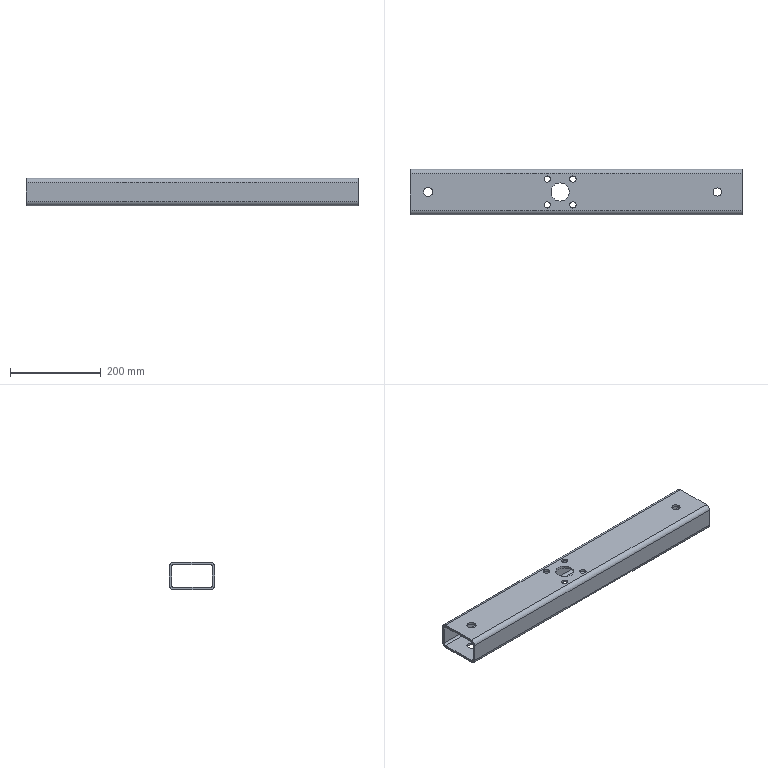Part | SolidWorks | features BaseBody 1 | 1 solid | 46 faces | box 730 x 100 x 60 mm | volume 1023592 mm3 | cylinder 36 | plane 10 | commonest cylinder face diameters 14 x16 20 x8 10 x4 18 x4 40 x4
STEP:
#1=CARTESIAN_POINT('',(30.,0.,-5.));
#2=VERTEX_POINT('',#1);
#3=CARTESIAN_POINT('',(50.,0.,-5.));
#4=VERTEX_POINT('',#3);
#5=CARTESIAN_POINT('',(40.,0.,-5.));
#6=DIRECTION('',(0.,0.,1.));
#7=DIRECTION('',(1.,0.,0.));
#8=AXIS2_PLACEMENT_3D('',#5,#6,#7);
#9=CIRCLE('',#8,10.);
#10=EDGE_CURVE('',#2,#4,#9,.T.);
#11=ORIENTED_EDGE('',*,*,#10,.F.);
#12=CARTESIAN_POINT('',(30.,0.,0.));
#13=VERTEX_POINT('',#12);
#14=CARTESIAN_POINT('',(30.,0.,-120.));
#15=DIRECTION('',(0.,0.,1.));
#16=VECTOR('',#15,1000.);
#17=LINE('',#14,#16);
#18=EDGE_CURVE('',#2,#13,#17,.T.);
#19=ORIENTED_EDGE('',*,*,#18,.T.);
#20=CARTESIAN_POINT('',(50.,0.,0.));
#21=VERTEX_POINT('',#20);
#22=CARTESIAN_POINT('',(40.,0.,0.));
#23=DIRECTION('',(0.,0.,1.));
#24=DIRECTION('',(1.,0.,0.));
#25=AXIS2_PLACEMENT_3D('',#22,#23,#24);
#26=CIRCLE('',#25,10.);
#27=EDGE_CURVE('',#13,#21,#26,.T.);
#28=ORIENTED_EDGE('',*,*,#27,.T.);
#29=CARTESIAN_POINT('',(50.,0.,-120.));
#30=DIRECTION('',(0.,0.,1.));
#31=VECTOR('',#30,1000.);
#32=LINE('',#29,#31);
#33=EDGE_CURVE('',#4,#21,#32,.T.);
#34=ORIENTED_EDGE('',*,*,#33,.F.);
#35=EDGE_LOOP('',(#11,#19,#28,#34));
#36=FACE_OUTER_BOUND('',#35,.T.);
#37=CARTESIAN_POINT('',(40.,0.,-120.));
#38=DIRECTION('',(0.,0.,1.));
#39=DIRECTION('',(1.,0.,0.));
#40=AXIS2_PLACEMENT_3D('',#37,#38,#39);
#41=CYLINDRICAL_SURFACE('',#40,10.);
#42=ADVANCED_FACE('',(#36),#41,.F.);
#43=CARTESIAN_POINT('',(675.708,9.,0.));
#44=VERTEX_POINT('',#43);
#45=CARTESIAN_POINT('',(675.708,-9.,0.));
#46=VERTEX_POINT('',#45);
#47=CARTESIAN_POINT('',(675.708,0.,0.));
#48=DIRECTION('',(0.,0.,1.));
#49=DIRECTION('',(0.,1.,0.));
#50=AXIS2_PLACEMENT_3D('',#47,#48,#49);
#51=CIRCLE('',#50,9.);
#52=EDGE_CURVE('',#44,#46,#51,.T.);
#53=ORIENTED_EDGE('',*,*,#52,.T.);
#54=CARTESIAN_POINT('',(675.708,-9.,-5.));
#55=VERTEX_POINT('',#54);
#56=CARTESIAN_POINT('',(675.708,-9.,56.));
#57=DIRECTION('',(0.,0.,-1.));
#58=VECTOR('',#57,1000.);
#59=LINE('',#56,#58);
#60=EDGE_CURVE('',#46,#55,#59,.T.);
#61=ORIENTED_EDGE('',*,*,#60,.T.);
#62=CARTESIAN_POINT('',(675.708,9.,-5.));
#63=VERTEX_POINT('',#62);
#64=CARTESIAN_POINT('',(675.708,0.,-5.));
#65=DIRECTION('',(0.,0.,1.));
#66=DIRECTION('',(0.,1.,0.));
#67=AXIS2_PLACEMENT_3D('',#64,#65,#66);
#68=CIRCLE('',#67,9.);
#69=EDGE_CURVE('',#63,#55,#68,.T.);
#70=ORIENTED_EDGE('',*,*,#69,.F.);
#71=CARTESIAN_POINT('',(675.708,9.,56.));
#72=DIRECTION('',(0.,0.,-1.));
#73=VECTOR('',#72,1000.);
#74=LINE('',#71,#73);
#75=EDGE_CURVE('',#44,#63,#74,.T.);
#76=ORIENTED_EDGE('',*,*,#75,.F.);
#77=EDGE_LOOP('',(#53,#61,#70,#76));
#78=FACE_OUTER_BOUND('',#77,.T.);
#79=CARTESIAN_POINT('',(675.708,0.,56.));
#80=DIRECTION('',(0.,0.,-1.));
#81=DIRECTION('',(0.,1.,0.));
#82=AXIS2_PLACEMENT_3D('',#79,#80,#81);
#83=CYLINDRICAL_SURFACE('',#82,9.);
#84=ADVANCED_FACE('',(#78),#83,.F.);
#85=CARTESIAN_POINT('',(330.,20.,0.));
#86=VERTEX_POINT('',#85);
#87=CARTESIAN_POINT('',(330.,-20.,0.));
#88=VERTEX_POINT('',#87);
#89=CARTESIAN_POINT('',(330.,0.,0.));
#90=DIRECTION('',(0.,0.,1.));
#91=DIRECTION('',(0.,1.,0.));
#92=AXIS2_PLACEMENT_3D('',#89,#90,#91);
#93=CIRCLE('',#92,20.);
#94=EDGE_CURVE('',#86,#88,#93,.T.);
#95=ORIENTED_EDGE('',*,*,#94,.T.);
#96=CARTESIAN_POINT('',(330.,-20.,-5.));
#97=VERTEX_POINT('',#96);
#98=CARTESIAN_POINT('',(330.,-20.,0.));
#99=DIRECTION('',(0.,0.,-1.));
#100=VECTOR('',#99,1000.);
#101=LINE('',#98,#100);
#102=EDGE_CURVE('',#88,#97,#101,.T.);
#103=ORIENTED_EDGE('',*,*,#102,.T.);
#104=CARTESIAN_POINT('',(330.,20.,-5.));
#105=VERTEX_POINT('',#104);
#106=CARTESIAN_POINT('',(330.,0.,-5.));
#107=DIRECTION('',(0.,0.,1.));
#108=DIRECTION('',(0.,1.,0.));
#109=AXIS2_PLACEMENT_3D('',#106,#107,#108);
#110=CIRCLE('',#109,20.);
#111=EDGE_CURVE('',#105,#97,#110,.T.);
#112=ORIENTED_EDGE('',*,*,#111,.F.);
#113=CARTESIAN_POINT('',(330.,20.,0.));
#114=DIRECTION('',(0.,0.,-1.));
#115=VECTOR('',#114,1000.);
#116=LINE('',#113,#115);
#117=EDGE_CURVE('',#86,#105,#116,.T.);
#118=ORIENTED_EDGE('',*,*,#117,.F.);
#119=EDGE_LOOP('',(#95,#103,#112,#118));
#120=FACE_OUTER_BOUND('',#119,.T.);
#121=CARTESIAN_POINT('',(330.,0.,0.));
#122=DIRECTION('',(0.,0.,-1.));
#123=DIRECTION('',(0.,1.,0.));
#124=AXIS2_PLACEMENT_3D('',#121,#122,#123);
#125=CYLINDRICAL_SURFACE('',#124,20.);
#126=ADVANCED_FACE('',(#120),#125,.F.);
#127=CARTESIAN_POINT('',(358.284,35.284,0.));
#128=VERTEX_POINT('',#127);
#129=CARTESIAN_POINT('',(358.284,21.284,0.));
#130=VERTEX_POINT('',#129);
#131=CARTESIAN_POINT('',(358.284,28.284,0.));
#132=DIRECTION('',(0.,0.,1.));
#133=DIRECTION('',(0.,1.,0.));
#134=AXIS2_PLACEMENT_3D('',#131,#132,#133);
#135=CIRCLE('',#134,7.);
#136=EDGE_CURVE('',#128,#130,#135,.T.);
#137=ORIENTED_EDGE('',*,*,#136,.T.);
#138=CARTESIAN_POINT('',(358.284,21.284,-5.));
#139=VERTEX_POINT('',#138);
#140=CARTESIAN_POINT('',(358.284,21.284,13.));
#141=DIRECTION('',(0.,0.,-1.));
#142=VECTOR('',#141,1000.);
#143=LINE('',#140,#142);
#144=EDGE_CURVE('',#130,#139,#143,.T.);
#145=ORIENTED_EDGE('',*,*,#144,.T.);
#146=CARTESIAN_POINT('',(358.284,35.284,-5.));
#147=VERTEX_POINT('',#146);
#148=CARTESIAN_POINT('',(358.284,28.284,-5.));
#149=DIRECTION('',(0.,0.,1.));
#150=DIRECTION('',(0.,1.,0.));
#151=AXIS2_PLACEMENT_3D('',#148,#149,#150);
#152=CIRCLE('',#151,7.);
#153=EDGE_CURVE('',#147,#139,#152,.T.);
#154=ORIENTED_EDGE('',*,*,#153,.F.);
#155=CARTESIAN_POINT('',(358.284,35.284,13.));
#156=DIRECTION('',(0.,0.,-1.));
#157=VECTOR('',#156,1000.);
#158=LINE('',#155,#157);
#159=EDGE_CURVE('',#128,#147,#158,.T.);
#160=ORIENTED_EDGE('',*,*,#159,.F.);
#161=EDGE_LOOP('',(#137,#145,#154,#160));
#162=FACE_OUTER_BOUND('',#161,.T.);
#163=CARTESIAN_POINT('',(358.284,28.284,13.));
#164=DIRECTION('',(0.,0.,-1.));
#165=DIRECTION('',(0.,1.,0.));
#166=AXIS2_PLACEMENT_3D('',#163,#164,#165);
#167=CYLINDRICAL_SURFACE('',#166,7.);
#168=ADVANCED_FACE('',(#162),#167,.F.);
#169=CARTESIAN_POINT('',(301.716,35.284,0.));
#170=VERTEX_POINT('',#169);
#171=CARTESIAN_POINT('',(301.716,21.284,0.));
#172=VERTEX_POINT('',#171);
#173=CARTESIAN_POINT('',(301.716,28.284,0.));
#174=DIRECTION('',(0.,0.,1.));
#175=DIRECTION('',(0.,1.,0.));
#176=AXIS2_PLACEMENT_3D('',#173,#174,#175);
#177=CIRCLE('',#176,7.);
#178=EDGE_CURVE('',#170,#172,#177,.T.);
#179=ORIENTED_EDGE('',*,*,#178,.T.);
#180=CARTESIAN_POINT('',(301.716,21.284,-5.));
#181=VERTEX_POINT('',#180);
#182=CARTESIAN_POINT('',(301.716,21.284,13.));
#183=DIRECTION('',(0.,0.,-1.));
#184=VECTOR('',#183,1000.);
#185=LINE('',#182,#184);
#186=EDGE_CURVE('',#172,#181,#185,.T.);
#187=ORIENTED_EDGE('',*,*,#186,.T.);
#188=CARTESIAN_POINT('',(301.716,35.284,-5.));
#189=VERTEX_POINT('',#188);
#190=CARTESIAN_POINT('',(301.716,28.284,-5.));
#191=DIRECTION('',(0.,0.,1.));
#192=DIRECTION('',(0.,1.,0.));
#193=AXIS2_PLACEMENT_3D('',#190,#191,#192);
#194=CIRCLE('',#193,7.);
#195=EDGE_CURVE('',#189,#181,#194,.T.);
#196=ORIENTED_EDGE('',*,*,#195,.F.);
#197=CARTESIAN_POINT('',(301.716,35.284,13.));
#198=DIRECTION('',(0.,0.,-1.));
#199=VECTOR('',#198,1000.);
#200=LINE('',#197,#199);
#201=EDGE_CURVE('',#170,#189,#200,.T.);
#202=ORIENTED_EDGE('',*,*,#201,.F.);
#203=EDGE_LOOP('',(#179,#187,#196,#202));
#204=FACE_OUTER_BOUND('',#203,.T.);
#205=CARTESIAN_POINT('',(301.716,28.284,13.));
#206=DIRECTION('',(0.,0.,-1.));
#207=DIRECTION('',(0.,1.,0.));
#208=AXIS2_PLACEMENT_3D('',#205,#206,#207);
#209=CYLINDRICAL_SURFACE('',#208,7.);
#210=ADVANCED_FACE('',(#204),#209,.F.);
#211=CARTESIAN_POINT('',(301.716,-21.284,0.));
#212=VERTEX_POINT('',#211);
#213=CARTESIAN_POINT('',(301.716,-35.284,0.));
#214=VERTEX_POINT('',#213);
#215=CARTESIAN_POINT('',(301.716,-28.284,0.));
#216=DIRECTION('',(0.,0.,1.));
#217=DIRECTION('',(0.,1.,0.));
#218=AXIS2_PLACEMENT_3D('',#215,#216,#217);
#219=CIRCLE('',#218,7.);
#220=EDGE_CURVE('',#212,#214,#219,.T.);
#221=ORIENTED_EDGE('',*,*,#220,.T.);
#222=CARTESIAN_POINT('',(301.716,-35.284,-5.));
#223=VERTEX_POINT('',#222);
#224=CARTESIAN_POINT('',(301.716,-35.284,13.));
#225=DIRECTION('',(0.,0.,-1.));
#226=VECTOR('',#225,1000.);
#227=LINE('',#224,#226);
#228=EDGE_CURVE('',#214,#223,#227,.T.);
#229=ORIENTED_EDGE('',*,*,#228,.T.);
#230=CARTESIAN_POINT('',(301.716,-21.284,-5.));
#231=VERTEX_POINT('',#230);
#232=CARTESIAN_POINT('',(301.716,-28.284,-5.));
#233=DIRECTION('',(0.,0.,1.));
#234=DIRECTION('',(0.,1.,0.));
#235=AXIS2_PLACEMENT_3D('',#232,#233,#234);
#236=CIRCLE('',#235,7.);
#237=EDGE_CURVE('',#231,#223,#236,.T.);
#238=ORIENTED_EDGE('',*,*,#237,.F.);
#239=CARTESIAN_POINT('',(301.716,-21.284,13.));
#240=DIRECTION('',(0.,0.,-1.));
#241=VECTOR('',#240,1000.);
#242=LINE('',#239,#241);
#243=EDGE_CURVE('',#212,#231,#242,.T.);
#244=ORIENTED_EDGE('',*,*,#243,.F.);
#245=EDGE_LOOP('',(#221,#229,#238,#244));
#246=FACE_OUTER_BOUND('',#245,.T.);
#247=CARTESIAN_POINT('',(301.716,-28.284,13.));
#248=DIRECTION('',(0.,0.,-1.));
#249=DIRECTION('',(0.,1.,0.));
#250=AXIS2_PLACEMENT_3D('',#247,#248,#249);
#251=CYLINDRICAL_SURFACE('',#250,7.);
#252=ADVANCED_FACE('',(#246),#251,.F.);
#253=CARTESIAN_POINT('',(358.284,-21.284,0.));
#254=VERTEX_POINT('',#253);
#255=CARTESIAN_POINT('',(358.284,-35.284,0.));
#256=VERTEX_POINT('',#255);
#257=CARTESIAN_POINT('',(358.284,-28.284,0.));
#258=DIRECTION('',(0.,0.,1.));
#259=DIRECTION('',(0.,1.,0.));
#260=AXIS2_PLACEMENT_3D('',#257,#258,#259);
#261=CIRCLE('',#260,7.);
#262=EDGE_CURVE('',#254,#256,#261,.T.);
#263=ORIENTED_EDGE('',*,*,#262,.T.);
#264=CARTESIAN_POINT('',(358.284,-35.284,-5.));
#265=VERTEX_POINT('',#264);
#266=CARTESIAN_POINT('',(358.284,-35.284,13.));
#267=DIRECTION('',(0.,0.,-1.));
#268=VECTOR('',#267,1000.);
#269=LINE('',#266,#268);
#270=EDGE_CURVE('',#256,#265,#269,.T.);
#271=ORIENTED_EDGE('',*,*,#270,.T.);
#272=CARTESIAN_POINT('',(358.284,-21.284,-5.));
#273=VERTEX_POINT('',#272);
#274=CARTESIAN_POINT('',(358.284,-28.284,-5.));
#275=DIRECTION('',(0.,0.,1.));
#276=DIRECTION('',(0.,1.,0.));
#277=AXIS2_PLACEMENT_3D('',#274,#275,#276);
#278=CIRCLE('',#277,7.);
#279=EDGE_CURVE('',#273,#265,#278,.T.);
#280=ORIENTED_EDGE('',*,*,#279,.F.);
#281=CARTESIAN_POINT('',(358.284,-21.284,13.));
#282=DIRECTION('',(0.,0.,-1.));
#283=VECTOR('',#282,1000.);
#284=LINE('',#281,#283);
#285=EDGE_CURVE('',#254,#273,#284,.T.);
#286=ORIENTED_EDGE('',*,*,#285,.F.);
#287=EDGE_LOOP('',(#263,#271,#280,#286));
#288=FACE_OUTER_BOUND('',#287,.T.);
#289=CARTESIAN_POINT('',(358.284,-28.284,13.));
#290=DIRECTION('',(0.,0.,-1.));
#291=DIRECTION('',(0.,1.,0.));
#292=AXIS2_PLACEMENT_3D('',#289,#290,#291);
#293=CYLINDRICAL_SURFACE('',#292,7.);
#294=ADVANCED_FACE('',(#288),#293,.F.);
#295=CARTESIAN_POINT('',(50.,0.,-60.));
#296=VERTEX_POINT('',#295);
#297=CARTESIAN_POINT('',(30.,0.,-60.));
#298=VERTEX_POINT('',#297);
#299=CARTESIAN_POINT('',(40.,0.,-60.));
#300=DIRECTION('',(0.,0.,-1.));
#301=DIRECTION('',(1.,0.,0.));
#302=AXIS2_PLACEMENT_3D('',#299,#300,#301);
#303=CIRCLE('',#302,10.);
#304=EDGE_CURVE('',#296,#298,#303,.T.);
#305=ORIENTED_EDGE('',*,*,#304,.T.);
#306=CARTESIAN_POINT('',(30.,0.,-55.));
#307=VERTEX_POINT('',#306);
#308=CARTESIAN_POINT('',(30.,0.,-120.));
#309=DIRECTION('',(0.,0.,1.));
#310=VECTOR('',#309,1000.);
#311=LINE('',#308,#310);
#312=EDGE_CURVE('',#298,#307,#311,.T.);
#313=ORIENTED_EDGE('',*,*,#312,.T.);
#314=CARTESIAN_POINT('',(50.,0.,-55.));
#315=VERTEX_POINT('',#314);
#316=CARTESIAN_POINT('',(40.,0.,-55.));
#317=DIRECTION('',(0.,0.,-1.));
#318=DIRECTION('',(1.,0.,0.));
#319=AXIS2_PLACEMENT_3D('',#316,#317,#318);
#320=CIRCLE('',#319,10.);
#321=EDGE_CURVE('',#315,#307,#320,.T.);
#322=ORIENTED_EDGE('',*,*,#321,.F.);
#323=CARTESIAN_POINT('',(50.,0.,-120.));
#324=DIRECTION('',(0.,0.,1.));
#325=VECTOR('',#324,1000.);
#326=LINE('',#323,#325);
#327=EDGE_CURVE('',#296,#315,#326,.T.);
#328=ORIENTED_EDGE('',*,*,#327,.F.);
#329=EDGE_LOOP('',(#305,#313,#322,#328));
#330=FACE_OUTER_BOUND('',#329,.T.);
#331=CARTESIAN_POINT('',(40.,0.,-120.));
#332=DIRECTION('',(0.,0.,1.));
#333=DIRECTION('',(1.,0.,0.));
#334=AXIS2_PLACEMENT_3D('',#331,#332,#333);
#335=CYLINDRICAL_SURFACE('',#334,10.);
#336=ADVANCED_FACE('',(#330),#335,.F.);
#337=CARTESIAN_POINT('',(675.708,-9.,-55.));
#338=VERTEX_POINT('',#337);
#339=CARTESIAN_POINT('',(675.708,9.,-55.));
#340=VERTEX_POINT('',#339);
#341=CARTESIAN_POINT('',(675.708,0.,-55.));
#342=DIRECTION('',(0.,0.,-1.));
#343=DIRECTION('',(0.,1.,0.));
#344=AXIS2_PLACEMENT_3D('',#341,#342,#343);
#345=CIRCLE('',#344,9.);
#346=EDGE_CURVE('',#338,#340,#345,.T.);
#347=ORIENTED_EDGE('',*,*,#346,.F.);
#348=CARTESIAN_POINT('',(675.708,-9.,-60.));
#349=VERTEX_POINT('',#348);
#350=CARTESIAN_POINT('',(675.708,-9.,56.));
#351=DIRECTION('',(0.,0.,-1.));
#352=VECTOR('',#351,1000.);
#353=LINE('',#350,#352);
#354=EDGE_CURVE('',#338,#349,#353,.T.);
#355=ORIENTED_EDGE('',*,*,#354,.T.);
#356=CARTESIAN_POINT('',(675.708,9.,-60.));
#357=VERTEX_POINT('',#356);
#358=CARTESIAN_POINT('',(675.708,0.,-60.));
#359=DIRECTION('',(0.,0.,-1.));
#360=DIRECTION('',(0.,1.,0.));
#361=AXIS2_PLACEMENT_3D('',#358,#359,#360);
#362=CIRCLE('',#361,9.);
#363=EDGE_CURVE('',#349,#357,#362,.T.);
#364=ORIENTED_EDGE('',*,*,#363,.T.);
#365=CARTESIAN_POINT('',(675.708,9.,56.));
#366=DIRECTION('',(0.,0.,-1.));
#367=VECTOR('',#366,1000.);
#368=LINE('',#365,#367);
#369=EDGE_CURVE('',#340,#357,#368,.T.);
#370=ORIENTED_EDGE('',*,*,#369,.F.);
#371=EDGE_LOOP('',(#347,#355,#364,#370));
#372=FACE_OUTER_BOUND('',#371,.T.);
#373=CARTESIAN_POINT('',(675.708,0.,56.));
#374=DIRECTION('',(0.,0.,-1.));
#375=DIRECTION('',(0.,1.,0.));
#376=AXIS2_PLACEMENT_3D('',#373,#374,#375);
#377=CYLINDRICAL_SURFACE('',#376,9.);
#378=ADVANCED_FACE('',(#372),#377,.F.);
#379=CARTESIAN_POINT('',(330.,-20.,-55.));
#380=VERTEX_POINT('',#379);
#381=CARTESIAN_POINT('',(330.,20.,-55.));
#382=VERTEX_POINT('',#381);
#383=CARTESIAN_POINT('',(330.,0.,-55.));
#384=DIRECTION('',(0.,0.,-1.));
#385=DIRECTION('',(0.,1.,0.));
#386=AXIS2_PLACEMENT_3D('',#383,#384,#385);
#387=CIRCLE('',#386,20.);
#388=EDGE_CURVE('',#380,#382,#387,.T.);
#389=ORIENTED_EDGE('',*,*,#388,.F.);
#390=CARTESIAN_POINT('',(330.,-20.,-60.));
#391=VERTEX_POINT('',#390);
#392=CARTESIAN_POINT('',(330.,-20.,0.));
#393=DIRECTION('',(0.,0.,-1.));
#394=VECTOR('',#393,1000.);
#395=LINE('',#392,#394);
#396=EDGE_CURVE('',#380,#391,#395,.T.);
#397=ORIENTED_EDGE('',*,*,#396,.T.);
#398=CARTESIAN_POINT('',(330.,20.,-60.));
#399=VERTEX_POINT('',#398);
#400=CARTESIAN_POINT('',(330.,0.,-60.));
#401=DIRECTION('',(0.,0.,-1.));
#402=DIRECTION('',(0.,1.,0.));
#403=AXIS2_PLACEMENT_3D('',#400,#401,#402);
#404=CIRCLE('',#403,20.);
#405=EDGE_CURVE('',#391,#399,#404,.T.);
#406=ORIENTED_EDGE('',*,*,#405,.T.);
#407=CARTESIAN_POINT('',(330.,20.,0.));
#408=DIRECTION('',(0.,0.,-1.));
#409=VECTOR('',#408,1000.);
#410=LINE('',#407,#409);
#411=EDGE_CURVE('',#382,#399,#410,.T.);
#412=ORIENTED_EDGE('',*,*,#411,.F.);
#413=EDGE_LOOP('',(#389,#397,#406,#412));
#414=FACE_OUTER_BOUND('',#413,.T.);
#415=CARTESIAN_POINT('',(330.,0.,0.));
#416=DIRECTION('',(0.,0.,-1.));
#417=DIRECTION('',(0.,1.,0.));
#418=AXIS2_PLACEMENT_3D('',#415,#416,#417);
#419=CYLINDRICAL_SURFACE('',#418,20.);
#420=ADVANCED_FACE('',(#414),#419,.F.);
#421=CARTESIAN_POINT('',(358.284,21.284,-55.));
#422=VERTEX_POINT('',#421);
#423=CARTESIAN_POINT('',(358.284,35.284,-55.));
#424=VERTEX_POINT('',#423);
#425=CARTESIAN_POINT('',(358.284,28.284,-55.));
#426=DIRECTION('',(0.,0.,-1.));
#427=DIRECTION('',(0.,1.,0.));
#428=AXIS2_PLACEMENT_3D('',#425,#426,#427);
#429=CIRCLE('',#428,7.);
#430=EDGE_CURVE('',#422,#424,#429,.T.);
#431=ORIENTED_EDGE('',*,*,#430,.F.);
#432=CARTESIAN_POINT('',(358.284,21.284,-60.));
#433=VERTEX_POINT('',#432);
#434=CARTESIAN_POINT('',(358.284,21.284,13.));
#435=DIRECTION('',(0.,0.,-1.));
#436=VECTOR('',#435,1000.);
#437=LINE('',#434,#436);
#438=EDGE_CURVE('',#422,#433,#437,.T.);
#439=ORIENTED_EDGE('',*,*,#438,.T.);
#440=CARTESIAN_POINT('',(358.284,35.284,-60.));
#441=VERTEX_POINT('',#440);
#442=CARTESIAN_POINT('',(358.284,28.284,-60.));
#443=DIRECTION('',(0.,0.,-1.));
#444=DIRECTION('',(0.,1.,0.));
#445=AXIS2_PLACEMENT_3D('',#442,#443,#444);
#446=CIRCLE('',#445,7.);
#447=EDGE_CURVE('',#433,#441,#446,.T.);
#448=ORIENTED_EDGE('',*,*,#447,.T.);
#449=CARTESIAN_POINT('',(358.284,35.284,13.));
#450=DIRECTION('',(0.,0.,-1.));
#451=VECTOR('',#450,1000.);
#452=LINE('',#449,#451);
#453=EDGE_CURVE('',#424,#441,#452,.T.);
#454=ORIENTED_EDGE('',*,*,#453,.F.);
#455=EDGE_LOOP('',(#431,#439,#448,#454));
#456=FACE_OUTER_BOUND('',#455,.T.);
#457=CARTESIAN_POINT('',(358.284,28.284,13.));
#458=DIRECTION('',(0.,0.,-1.));
#459=DIRECTION('',(0.,1.,0.));
#460=AXIS2_PLACEMENT_3D('',#457,#458,#459);
#461=CYLINDRICAL_SURFACE('',#460,7.);
#462=ADVANCED_FACE('',(#456),#461,.F.);
#463=CARTESIAN_POINT('',(301.716,21.284,-55.));
#464=VERTEX_POINT('',#463);
#465=CARTESIAN_POINT('',(301.716,35.284,-55.));
#466=VERTEX_POINT('',#465);
#467=CARTESIAN_POINT('',(301.716,28.284,-55.));
#468=DIRECTION('',(0.,0.,-1.));
#469=DIRECTION('',(0.,1.,0.));
#470=AXIS2_PLACEMENT_3D('',#467,#468,#469);
#471=CIRCLE('',#470,7.);
#472=EDGE_CURVE('',#464,#466,#471,.T.);
#473=ORIENTED_EDGE('',*,*,#472,.F.);
#474=CARTESIAN_POINT('',(301.716,21.284,-60.));
#475=VERTEX_POINT('',#474);
#476=CARTESIAN_POINT('',(301.716,21.284,13.));
#477=DIRECTION('',(0.,0.,-1.));
#478=VECTOR('',#477,1000.);
#479=LINE('',#476,#478);
#480=EDGE_CURVE('',#464,#475,#479,.T.);
#481=ORIENTED_EDGE('',*,*,#480,.T.);
#482=CARTESIAN_POINT('',(301.716,35.284,-60.));
#483=VERTEX_POINT('',#482);
#484=CARTESIAN_POINT('',(301.716,28.284,-60.));
#485=DIRECTION('',(0.,0.,-1.));
#486=DIRECTION('',(0.,1.,0.));
#487=AXIS2_PLACEMENT_3D('',#484,#485,#486);
#488=CIRCLE('',#487,7.);
#489=EDGE_CURVE('',#475,#483,#488,.T.);
#490=ORIENTED_EDGE('',*,*,#489,.T.);
#491=CARTESIAN_POINT('',(301.716,35.284,13.));
#492=DIRECTION('',(0.,0.,-1.));
#493=VECTOR('',#492,1000.);
#494=LINE('',#491,#493);
#495=EDGE_CURVE('',#466,#483,#494,.T.);
#496=ORIENTED_EDGE('',*,*,#495,.F.);
#497=EDGE_LOOP('',(#473,#481,#490,#496));
#498=FACE_OUTER_BOUND('',#497,.T.);
#499=CARTESIAN_POINT('',(301.716,28.284,13.));
#500=DIRECTION('',(0.,0.,-1.));
#501=DIRECTION('',(0.,1.,0.));
#502=AXIS2_PLACEMENT_3D('',#499,#500,#501);
#503=CYLINDRICAL_SURFACE('',#502,7.);
#504=ADVANCED_FACE('',(#498),#503,.F.);
#505=CARTESIAN_POINT('',(301.716,-35.284,-55.));
#506=VERTEX_POINT('',#505);
#507=CARTESIAN_POINT('',(301.716,-21.284,-55.));
#508=VERTEX_POINT('',#507);
#509=CARTESIAN_POINT('',(301.716,-28.284,-55.));
#510=DIRECTION('',(0.,0.,-1.));
#511=DIRECTION('',(0.,1.,0.));
#512=AXIS2_PLACEMENT_3D('',#509,#510,#511);
#513=CIRCLE('',#512,7.);
#514=EDGE_CURVE('',#506,#508,#513,.T.);
#515=ORIENTED_EDGE('',*,*,#514,.F.);
#516=CARTESIAN_POINT('',(301.716,-35.284,-60.));
#517=VERTEX_POINT('',#516);
#518=CARTESIAN_POINT('',(301.716,-35.284,13.));
#519=DIRECTION('',(0.,0.,-1.));
#520=VECTOR('',#519,1000.);
#521=LINE('',#518,#520);
#522=EDGE_CURVE('',#506,#517,#521,.T.);
#523=ORIENTED_EDGE('',*,*,#522,.T.);
#524=CARTESIAN_POINT('',(301.716,-21.284,-60.));
#525=VERTEX_POINT('',#524);
#526=CARTESIAN_POINT('',(301.716,-28.284,-60.));
#527=DIRECTION('',(0.,0.,-1.));
#528=DIRECTION('',(0.,1.,0.));
#529=AXIS2_PLACEMENT_3D('',#526,#527,#528);
#530=CIRCLE('',#529,7.);
#531=EDGE_CURVE('',#517,#525,#530,.T.);
#532=ORIENTED_EDGE('',*,*,#531,.T.);
#533=CARTESIAN_POINT('',(301.716,-21.284,13.));
#534=DIRECTION('',(0.,0.,-1.));
#535=VECTOR('',#534,1000.);
#536=LINE('',#533,#535);
#537=EDGE_CURVE('',#508,#525,#536,.T.);
#538=ORIENTED_EDGE('',*,*,#537,.F.);
#539=EDGE_LOOP('',(#515,#523,#532,#538));
#540=FACE_OUTER_BOUND('',#539,.T.);
#541=CARTESIAN_POINT('',(301.716,-28.284,13.));
#542=DIRECTION('',(0.,0.,-1.));
#543=DIRECTION('',(0.,1.,0.));
#544=AXIS2_PLACEMENT_3D('',#541,#542,#543);
#545=CYLINDRICAL_SURFACE('',#544,7.);
#546=ADVANCED_FACE('',(#540),#545,.F.);
#547=CARTESIAN_POINT('',(358.284,-35.284,-55.));
#548=VERTEX_POINT('',#547);
#549=CARTESIAN_POINT('',(358.284,-21.284,-55.));
#550=VERTEX_POINT('',#549);
#551=CARTESIAN_POINT('',(358.284,-28.284,-55.));
#552=DIRECTION('',(0.,0.,-1.));
#553=DIRECTION('',(0.,1.,0.));
#554=AXIS2_PLACEMENT_3D('',#551,#552,#553);
#555=CIRCLE('',#554,7.);
#556=EDGE_CURVE('',#548,#550,#555,.T.);
#557=ORIENTED_EDGE('',*,*,#556,.F.);
#558=CARTESIAN_POINT('',(358.284,-35.284,-60.));
#559=VERTEX_POINT('',#558);
#560=CARTESIAN_POINT('',(358.284,-35.284,13.));
#561=DIRECTION('',(0.,0.,-1.));
#562=VECTOR('',#561,1000.);
#563=LINE('',#560,#562);
#564=EDGE_CURVE('',#548,#559,#563,.T.);
#565=ORIENTED_EDGE('',*,*,#564,.T.);
#566=CARTESIAN_POINT('',(358.284,-21.284,-60.));
#567=VERTEX_POINT('',#566);
#568=CARTESIAN_POINT('',(358.284,-28.284,-60.));
#569=DIRECTION('',(0.,0.,-1.));
#570=DIRECTION('',(0.,1.,0.));
#571=AXIS2_PLACEMENT_3D('',#568,#569,#570);
#572=CIRCLE('',#571,7.);
#573=EDGE_CURVE('',#559,#567,#572,.T.);
#574=ORIENTED_EDGE('',*,*,#573,.T.);
#575=CARTESIAN_POINT('',(358.284,-21.284,13.));
#576=DIRECTION('',(0.,0.,-1.));
#577=VECTOR('',#576,1000.);
#578=LINE('',#575,#577);
#579=EDGE_CURVE('',#550,#567,#578,.T.);
#580=ORIENTED_EDGE('',*,*,#579,.F.);
#581=EDGE_LOOP('',(#557,#565,#574,#580));
#582=FACE_OUTER_BOUND('',#581,.T.);
#583=CARTESIAN_POINT('',(358.284,-28.284,13.));
#584=DIRECTION('',(0.,0.,-1.));
#585=DIRECTION('',(0.,1.,0.));
#586=AXIS2_PLACEMENT_3D('',#583,#584,#585);
#587=CYLINDRICAL_SURFACE('',#586,7.);
#588=ADVANCED_FACE('',(#582),#587,.F.);
#589=CARTESIAN_POINT('',(730.,-40.,0.));
#590=VERTEX_POINT('',#589);
#591=CARTESIAN_POINT('',(0.,-40.,0.));
#592=VERTEX_POINT('',#591);
#593=CARTESIAN_POINT('',(730.,-40.,0.));
#594=DIRECTION('',(-1.,0.,0.));
#595=VECTOR('',#594,1000.);
#596=LINE('',#593,#595);
#597=EDGE_CURVE('',#590,#592,#596,.T.);
#598=ORIENTED_EDGE('',*,*,#597,.F.);
#599=CARTESIAN_POINT('',(730.,40.,0.));
#600=VERTEX_POINT('',#599);
#601=CARTESIAN_POINT('',(730.,-40.,0.));
#602=DIRECTION('',(0.,-1.,0.));
#603=VECTOR('',#602,1000.);
#604=LINE('',#601,#603);
#605=EDGE_CURVE('',#600,#590,#604,.T.);
#606=ORIENTED_EDGE('',*,*,#605,.F.);
#607=CARTESIAN_POINT('',(0.,40.,0.));
#608=VERTEX_POINT('',#607);
#609=CARTESIAN_POINT('',(730.,40.,0.));
#610=DIRECTION('',(1.,0.,0.));
#611=VECTOR('',#610,1000.);
#612=LINE('',#609,#611);
#613=EDGE_CURVE('',#608,#600,#612,.T.);
#614=ORIENTED_EDGE('',*,*,#613,.F.);
#615=CARTESIAN_POINT('',(0.,-40.,0.));
#616=DIRECTION('',(0.,1.,0.));
#617=VECTOR('',#616,1000.);
#618=LINE('',#615,#617);
#619=EDGE_CURVE('',#592,#608,#618,.T.);
#620=ORIENTED_EDGE('',*,*,#619,.F.);
#621=EDGE_LOOP('',(#598,#606,#614,#620));
#622=FACE_OUTER_BOUND('',#621,.T.);
#623=CARTESIAN_POINT('',(40.,0.,0.));
#624=DIRECTION('',(0.,0.,1.));
#625=DIRECTION('',(1.,0.,0.));
#626=AXIS2_PLACEMENT_3D('',#623,#624,#625);
#627=CIRCLE('',#626,10.);
#628=EDGE_CURVE('',#21,#13,#627,.T.);
#629=ORIENTED_EDGE('',*,*,#628,.F.);
#630=ORIENTED_EDGE('',*,*,#27,.F.);
#631=EDGE_LOOP('',(#629,#630));
#632=FACE_BOUND('',#631,.T.);
#633=ORIENTED_EDGE('',*,*,#52,.F.);
#634=CARTESIAN_POINT('',(675.708,0.,0.));
#635=DIRECTION('',(0.,0.,1.));
#636=DIRECTION('',(0.,1.,0.));
#637=AXIS2_PLACEMENT_3D('',#634,#635,#636);
#638=CIRCLE('',#637,9.);
#639=EDGE_CURVE('',#46,#44,#638,.T.);
#640=ORIENTED_EDGE('',*,*,#639,.F.);
#641=EDGE_LOOP('',(#633,#640));
#642=FACE_BOUND('',#641,.T.);
#643=ORIENTED_EDGE('',*,*,#94,.F.);
#644=CARTESIAN_POINT('',(330.,0.,0.));
#645=DIRECTION('',(0.,0.,1.));
#646=DIRECTION('',(0.,1.,0.));
#647=AXIS2_PLACEMENT_3D('',#644,#645,#646);
#648=CIRCLE('',#647,20.);
#649=EDGE_CURVE('',#88,#86,#648,.T.);
#650=ORIENTED_EDGE('',*,*,#649,.F.);
#651=EDGE_LOOP('',(#643,#650));
#652=FACE_BOUND('',#651,.T.);
#653=ORIENTED_EDGE('',*,*,#136,.F.);
#654=CARTESIAN_POINT('',(358.284,28.284,0.));
#655=DIRECTION('',(0.,0.,1.));
#656=DIRECTION('',(0.,1.,0.));
#657=AXIS2_PLACEMENT_3D('',#654,#655,#656);
#658=CIRCLE('',#657,7.);
#659=EDGE_CURVE('',#130,#128,#658,.T.);
#660=ORIENTED_EDGE('',*,*,#659,.F.);
#661=EDGE_LOOP('',(#653,#660));
#662=FACE_BOUND('',#661,.T.);
#663=ORIENTED_EDGE('',*,*,#178,.F.);
#664=CARTESIAN_POINT('',(301.716,28.284,0.));
#665=DIRECTION('',(0.,0.,1.));
#666=DIRECTION('',(0.,1.,0.));
#667=AXIS2_PLACEMENT_3D('',#664,#665,#666);
#668=CIRCLE('',#667,7.);
#669=EDGE_CURVE('',#172,#170,#668,.T.);
#670=ORIENTED_EDGE('',*,*,#669,.F.);
#671=EDGE_LOOP('',(#663,#670));
#672=FACE_BOUND('',#671,.T.);
#673=ORIENTED_EDGE('',*,*,#220,.F.);
#674=CARTESIAN_POINT('',(301.716,-28.284,0.));
#675=DIRECTION('',(0.,0.,1.));
#676=DIRECTION('',(0.,1.,0.));
#677=AXIS2_PLACEMENT_3D('',#674,#675,#676);
#678=CIRCLE('',#677,7.);
#679=EDGE_CURVE('',#214,#212,#678,.T.);
#680=ORIENTED_EDGE('',*,*,#679,.F.);
#681=EDGE_LOOP('',(#673,#680));
#682=FACE_BOUND('',#681,.T.);
#683=ORIENTED_EDGE('',*,*,#262,.F.);
#684=CARTESIAN_POINT('',(358.284,-28.284,0.));
#685=DIRECTION('',(0.,0.,1.));
#686=DIRECTION('',(0.,1.,0.));
#687=AXIS2_PLACEMENT_3D('',#684,#685,#686);
#688=CIRCLE('',#687,7.);
#689=EDGE_CURVE('',#256,#254,#688,.T.);
#690=ORIENTED_EDGE('',*,*,#689,.F.);
#691=EDGE_LOOP('',(#683,#690));
#692=FACE_BOUND('',#691,.T.);
#693=CARTESIAN_POINT('',(730.,-40.,0.));
#694=DIRECTION('',(0.,0.,-1.));
#695=DIRECTION('',(0.,1.,0.));
#696=AXIS2_PLACEMENT_3D('',#693,#694,#695);
#697=PLANE('',#696);
#698=ADVANCED_FACE('',(#622,#632,#642,#652,#662,#672,#682,#692),#697,.F.);
#699=ORIENTED_EDGE('',*,*,#619,.T.);
#700=CARTESIAN_POINT('',(0.,50.,-10.));
#701=VERTEX_POINT('',#700);
#702=CARTESIAN_POINT('',(0.,40.,-10.));
#703=DIRECTION('',(1.,0.,0.));
#704=DIRECTION('',(0.,0.,1.));
#705=AXIS2_PLACEMENT_3D('',#702,#703,#704);
#706=CIRCLE('',#705,10.);
#707=EDGE_CURVE('',#701,#608,#706,.T.);
#708=ORIENTED_EDGE('',*,*,#707,.F.);
#709=CARTESIAN_POINT('',(0.,50.,-50.));
#710=VERTEX_POINT('',#709);
#711=CARTESIAN_POINT('',(0.,50.,-10.));
#712=DIRECTION('',(0.,0.,1.));
#713=VECTOR('',#712,1000.);
#714=LINE('',#711,#713);
#715=EDGE_CURVE('',#710,#701,#714,.T.);
#716=ORIENTED_EDGE('',*,*,#715,.F.);
#717=CARTESIAN_POINT('',(0.,40.,-60.));
#718=VERTEX_POINT('',#717);
#719=CARTESIAN_POINT('',(0.,40.,-50.));
#720=DIRECTION('',(1.,0.,0.));
#721=DIRECTION('',(0.,0.,1.));
#722=AXIS2_PLACEMENT_3D('',#719,#720,#721);
#723=CIRCLE('',#722,10.);
#724=EDGE_CURVE('',#718,#710,#723,.T.);
#725=ORIENTED_EDGE('',*,*,#724,.F.);
#726=CARTESIAN_POINT('',(0.,-40.,-60.));
#727=VERTEX_POINT('',#726);
#728=CARTESIAN_POINT('',(0.,-40.,-60.));
#729=DIRECTION('',(0.,1.,0.));
#730=VECTOR('',#729,1000.);
#731=LINE('',#728,#730);
#732=EDGE_CURVE('',#727,#718,#731,.T.);
#733=ORIENTED_EDGE('',*,*,#732,.F.);
#734=CARTESIAN_POINT('',(0.,-50.,-50.));
#735=VERTEX_POINT('',#734);
#736=CARTESIAN_POINT('',(0.,-40.,-50.));
#737=DIRECTION('',(1.,0.,0.));
#738=DIRECTION('',(0.,0.,1.));
#739=AXIS2_PLACEMENT_3D('',#736,#737,#738);
#740=CIRCLE('',#739,10.);
#741=EDGE_CURVE('',#735,#727,#740,.T.);
#742=ORIENTED_EDGE('',*,*,#741,.F.);
#743=CARTESIAN_POINT('',(0.,-50.,-10.));
#744=VERTEX_POINT('',#743);
#745=CARTESIAN_POINT('',(0.,-50.,-10.));
#746=DIRECTION('',(0.,0.,-1.));
#747=VECTOR('',#746,1000.);
#748=LINE('',#745,#747);
#749=EDGE_CURVE('',#744,#735,#748,.T.);
#750=ORIENTED_EDGE('',*,*,#749,.F.);
#751=CARTESIAN_POINT('',(0.,-40.,-10.));
#752=DIRECTION('',(1.,0.,0.));
#753=DIRECTION('',(0.,0.,1.));
#754=AXIS2_PLACEMENT_3D('',#751,#752,#753);
#755=CIRCLE('',#754,10.);
#756=EDGE_CURVE('',#592,#744,#755,.T.);
#757=ORIENTED_EDGE('',*,*,#756,.F.);
#758=EDGE_LOOP('',(#699,#708,#716,#725,#733,#742,#750,#757));
#759=FACE_OUTER_BOUND('',#758,.T.);
#760=CARTESIAN_POINT('',(0.,40.,-55.));
#761=VERTEX_POINT('',#760);
#762=CARTESIAN_POINT('',(0.,-40.,-55.));
#763=VERTEX_POINT('',#762);
#764=CARTESIAN_POINT('',(0.,-40.,-55.));
#765=DIRECTION('',(0.,-1.,0.));
#766=VECTOR('',#765,1000.);
#767=LINE('',#764,#766);
#768=EDGE_CURVE('',#761,#763,#767,.T.);
#769=ORIENTED_EDGE('',*,*,#768,.F.);
#770=CARTESIAN_POINT('',(0.,45.,-50.));
#771=VERTEX_POINT('',#770);
#772=CARTESIAN_POINT('',(0.,40.,-50.));
#773=DIRECTION('',(-1.,0.,0.));
#774=DIRECTION('',(0.,0.,1.));
#775=AXIS2_PLACEMENT_3D('',#772,#773,#774);
#776=CIRCLE('',#775,5.);
#777=EDGE_CURVE('',#771,#761,#776,.T.);
#778=ORIENTED_EDGE('',*,*,#777,.F.);
#779=CARTESIAN_POINT('',(0.,45.,-10.));
#780=VERTEX_POINT('',#779);
#781=CARTESIAN_POINT('',(0.,45.,-10.));
#782=DIRECTION('',(0.,0.,-1.));
#783=VECTOR('',#782,1000.);
#784=LINE('',#781,#783);
#785=EDGE_CURVE('',#780,#771,#784,.T.);
#786=ORIENTED_EDGE('',*,*,#785,.F.);
#787=CARTESIAN_POINT('',(0.,40.,-5.));
#788=VERTEX_POINT('',#787);
#789=CARTESIAN_POINT('',(0.,40.,-10.));
#790=DIRECTION('',(-1.,0.,0.));
#791=DIRECTION('',(0.,0.,1.));
#792=AXIS2_PLACEMENT_3D('',#789,#790,#791);
#793=CIRCLE('',#792,5.);
#794=EDGE_CURVE('',#788,#780,#793,.T.);
#795=ORIENTED_EDGE('',*,*,#794,.F.);
#796=CARTESIAN_POINT('',(0.,-40.,-5.));
#797=VERTEX_POINT('',#796);
#798=CARTESIAN_POINT('',(0.,-40.,-5.));
#799=DIRECTION('',(0.,1.,0.));
#800=VECTOR('',#799,1000.);
#801=LINE('',#798,#800);
#802=EDGE_CURVE('',#797,#788,#801,.T.);
#803=ORIENTED_EDGE('',*,*,#802,.F.);
#804=CARTESIAN_POINT('',(0.,-45.,-10.));
#805=VERTEX_POINT('',#804);
#806=CARTESIAN_POINT('',(0.,-40.,-10.));
#807=DIRECTION('',(-1.,0.,0.));
#808=DIRECTION('',(0.,0.,1.));
#809=AXIS2_PLACEMENT_3D('',#806,#807,#808);
#810=CIRCLE('',#809,5.);
#811=EDGE_CURVE('',#805,#797,#810,.T.);
#812=ORIENTED_EDGE('',*,*,#811,.F.);
#813=CARTESIAN_POINT('',(0.,-45.,-50.));
#814=VERTEX_POINT('',#813);
#815=CARTESIAN_POINT('',(0.,-45.,-10.));
#816=DIRECTION('',(0.,0.,1.));
#817=VECTOR('',#816,1000.);
#818=LINE('',#815,#817);
#819=EDGE_CURVE('',#814,#805,#818,.T.);
#820=ORIENTED_EDGE('',*,*,#819,.F.);
#821=CARTESIAN_POINT('',(0.,-40.,-50.));
#822=DIRECTION('',(-1.,0.,0.));
#823=DIRECTION('',(0.,0.,1.));
#824=AXIS2_PLACEMENT_3D('',#821,#822,#823);
#825=CIRCLE('',#824,5.);
#826=EDGE_CURVE('',#763,#814,#825,.T.);
#827=ORIENTED_EDGE('',*,*,#826,.F.);
#828=EDGE_LOOP('',(#769,#778,#786,#795,#803,#812,#820,#827));
#829=FACE_BOUND('',#828,.T.);
#830=CARTESIAN_POINT('',(0.,-40.,-10.));
#831=DIRECTION('',(1.,0.,0.));
#832=DIRECTION('',(0.,0.,-1.));
#833=AXIS2_PLACEMENT_3D('',#830,#831,#832);
#834=PLANE('',#833);
#835=ADVANCED_FACE('',(#759,#829),#834,.F.);
#836=CARTESIAN_POINT('',(730.,-50.,-10.));
#837=VERTEX_POINT('',#836);
#838=CARTESIAN_POINT('',(730.,-40.,-10.));
#839=DIRECTION('',(-1.,0.,0.));
#840=DIRECTION('',(0.,0.,1.));
#841=AXIS2_PLACEMENT_3D('',#838,#839,#840);
#842=CIRCLE('',#841,10.);
#843=EDGE_CURVE('',#837,#590,#842,.T.);
#844=ORIENTED_EDGE('',*,*,#843,.T.);
#845=ORIENTED_EDGE('',*,*,#597,.T.);
#846=ORIENTED_EDGE('',*,*,#756,.T.);
#847=CARTESIAN_POINT('',(730.,-50.,-10.));
#848=DIRECTION('',(1.,0.,0.));
#849=VECTOR('',#848,1000.);
#850=LINE('',#847,#849);
#851=EDGE_CURVE('',#744,#837,#850,.T.);
#852=ORIENTED_EDGE('',*,*,#851,.T.);
#853=EDGE_LOOP('',(#844,#845,#846,#852));
#854=FACE_OUTER_BOUND('',#853,.T.);
#855=CARTESIAN_POINT('',(730.,-40.,-10.));
#856=DIRECTION('',(-1.,0.,0.));
#857=DIRECTION('',(0.,0.,1.));
#858=AXIS2_PLACEMENT_3D('',#855,#856,#857);
#859=CYLINDRICAL_SURFACE('',#858,10.);
#860=ADVANCED_FACE('',(#854),#859,.T.);
#861=CARTESIAN_POINT('',(730.,50.,-10.));
#862=VERTEX_POINT('',#861);
#863=CARTESIAN_POINT('',(730.,40.,-10.));
#864=DIRECTION('',(1.,0.,0.));
#865=DIRECTION('',(0.,0.,1.));
#866=AXIS2_PLACEMENT_3D('',#863,#864,#865);
#867=CIRCLE('',#866,10.);
#868=EDGE_CURVE('',#862,#600,#867,.T.);
#869=ORIENTED_EDGE('',*,*,#868,.T.);
#870=ORIENTED_EDGE('',*,*,#605,.T.);
#871=ORIENTED_EDGE('',*,*,#843,.F.);
#872=CARTESIAN_POINT('',(730.,-50.,-50.));
#873=VERTEX_POINT('',#872);
#874=CARTESIAN_POINT('',(730.,-50.,-10.));
#875=DIRECTION('',(0.,0.,-1.));
#876=VECTOR('',#875,1000.);
#877=LINE('',#874,#876);
#878=EDGE_CURVE('',#837,#873,#877,.T.);
#879=ORIENTED_EDGE('',*,*,#878,.T.);
#880=CARTESIAN_POINT('',(730.,-40.,-60.));
#881=VERTEX_POINT('',#880);
#882=CARTESIAN_POINT('',(730.,-40.,-50.));
#883=DIRECTION('',(1.,0.,0.));
#884=DIRECTION('',(0.,0.,1.));
#885=AXIS2_PLACEMENT_3D('',#882,#883,#884);
#886=CIRCLE('',#885,10.);
#887=EDGE_CURVE('',#873,#881,#886,.T.);
#888=ORIENTED_EDGE('',*,*,#887,.T.);
#889=CARTESIAN_POINT('',(730.,40.,-60.));
#890=VERTEX_POINT('',#889);
#891=CARTESIAN_POINT('',(730.,-40.,-60.));
#892=DIRECTION('',(0.,1.,0.));
#893=VECTOR('',#892,1000.);
#894=LINE('',#891,#893);
#895=EDGE_CURVE('',#881,#890,#894,.T.);
#896=ORIENTED_EDGE('',*,*,#895,.T.);
#897=CARTESIAN_POINT('',(730.,50.,-50.));
#898=VERTEX_POINT('',#897);
#899=CARTESIAN_POINT('',(730.,40.,-50.));
#900=DIRECTION('',(1.,0.,0.));
#901=DIRECTION('',(0.,0.,1.));
#902=AXIS2_PLACEMENT_3D('',#899,#900,#901);
#903=CIRCLE('',#902,10.);
#904=EDGE_CURVE('',#890,#898,#903,.T.);
#905=ORIENTED_EDGE('',*,*,#904,.T.);
#906=CARTESIAN_POINT('',(730.,50.,-10.));
#907=DIRECTION('',(0.,0.,1.));
#908=VECTOR('',#907,1000.);
#909=LINE('',#906,#908);
#910=EDGE_CURVE('',#898,#862,#909,.T.);
#911=ORIENTED_EDGE('',*,*,#910,.T.);
#912=EDGE_LOOP('',(#869,#870,#871,#879,#888,#896,#905,#911));
#913=FACE_OUTER_BOUND('',#912,.T.);
#914=CARTESIAN_POINT('',(730.,45.,-50.));
#915=VERTEX_POINT('',#914);
#916=CARTESIAN_POINT('',(730.,40.,-55.));
#917=VERTEX_POINT('',#916);
#918=CARTESIAN_POINT('',(730.,40.,-50.));
#919=DIRECTION('',(-1.,0.,0.));
#920=DIRECTION('',(0.,0.,1.));
#921=AXIS2_PLACEMENT_3D('',#918,#919,#920);
#922=CIRCLE('',#921,5.);
#923=EDGE_CURVE('',#915,#917,#922,.T.);
#924=ORIENTED_EDGE('',*,*,#923,.T.);
#925=CARTESIAN_POINT('',(730.,-40.,-55.));
#926=VERTEX_POINT('',#925);
#927=CARTESIAN_POINT('',(730.,-40.,-55.));
#928=DIRECTION('',(0.,-1.,0.));
#929=VECTOR('',#928,1000.);
#930=LINE('',#927,#929);
#931=EDGE_CURVE('',#917,#926,#930,.T.);
#932=ORIENTED_EDGE('',*,*,#931,.T.);
#933=CARTESIAN_POINT('',(730.,-45.,-50.));
#934=VERTEX_POINT('',#933);
#935=CARTESIAN_POINT('',(730.,-40.,-50.));
#936=DIRECTION('',(-1.,0.,0.));
#937=DIRECTION('',(0.,0.,1.));
#938=AXIS2_PLACEMENT_3D('',#935,#936,#937);
#939=CIRCLE('',#938,5.);
#940=EDGE_CURVE('',#926,#934,#939,.T.);
#941=ORIENTED_EDGE('',*,*,#940,.T.);
#942=CARTESIAN_POINT('',(730.,-45.,-10.));
#943=VERTEX_POINT('',#942);
#944=CARTESIAN_POINT('',(730.,-45.,-10.));
#945=DIRECTION('',(0.,0.,1.));
#946=VECTOR('',#945,1000.);
#947=LINE('',#944,#946);
#948=EDGE_CURVE('',#934,#943,#947,.T.);
#949=ORIENTED_EDGE('',*,*,#948,.T.);
#950=CARTESIAN_POINT('',(730.,-40.,-5.));
#951=VERTEX_POINT('',#950);
#952=CARTESIAN_POINT('',(730.,-40.,-10.));
#953=DIRECTION('',(-1.,0.,0.));
#954=DIRECTION('',(0.,0.,1.));
#955=AXIS2_PLACEMENT_3D('',#952,#953,#954);
#956=CIRCLE('',#955,5.);
#957=EDGE_CURVE('',#943,#951,#956,.T.);
#958=ORIENTED_EDGE('',*,*,#957,.T.);
#959=CARTESIAN_POINT('',(730.,40.,-5.));
#960=VERTEX_POINT('',#959);
#961=CARTESIAN_POINT('',(730.,-40.,-5.));
#962=DIRECTION('',(0.,1.,0.));
#963=VECTOR('',#962,1000.);
#964=LINE('',#961,#963);
#965=EDGE_CURVE('',#951,#960,#964,.T.);
#966=ORIENTED_EDGE('',*,*,#965,.T.);
#967=CARTESIAN_POINT('',(730.,45.,-10.));
#968=VERTEX_POINT('',#967);
#969=CARTESIAN_POINT('',(730.,40.,-10.));
#970=DIRECTION('',(-1.,0.,0.));
#971=DIRECTION('',(0.,0.,1.));
#972=AXIS2_PLACEMENT_3D('',#969,#970,#971);
#973=CIRCLE('',#972,5.);
#974=EDGE_CURVE('',#960,#968,#973,.T.);
#975=ORIENTED_EDGE('',*,*,#974,.T.);
#976=CARTESIAN_POINT('',(730.,45.,-10.));
#977=DIRECTION('',(0.,0.,-1.));
#978=VECTOR('',#977,1000.);
#979=LINE('',#976,#978);
#980=EDGE_CURVE('',#968,#915,#979,.T.);
#981=ORIENTED_EDGE('',*,*,#980,.T.);
#982=EDGE_LOOP('',(#924,#932,#941,#949,#958,#966,#975,#981));
#983=FACE_BOUND('',#982,.T.);
#984=CARTESIAN_POINT('',(730.,-40.,-10.));
#985=DIRECTION('',(1.,0.,0.));
#986=DIRECTION('',(0.,0.,-1.));
#987=AXIS2_PLACEMENT_3D('',#984,#985,#986);
#988=PLANE('',#987);
#989=ADVANCED_FACE('',(#913,#983),#988,.T.);
#990=ORIENTED_EDGE('',*,*,#868,.F.);
#991=CARTESIAN_POINT('',(730.,50.,-10.));
#992=DIRECTION('',(-1.,0.,0.));
#993=VECTOR('',#992,1000.);
#994=LINE('',#991,#993);
#995=EDGE_CURVE('',#862,#701,#994,.T.);
#996=ORIENTED_EDGE('',*,*,#995,.T.);
#997=ORIENTED_EDGE('',*,*,#707,.T.);
#998=ORIENTED_EDGE('',*,*,#613,.T.);
#999=EDGE_LOOP('',(#990,#996,#997,#998));
#1000=FACE_OUTER_BOUND('',#999,.T.);
#1001=CARTESIAN_POINT('',(730.,40.,-10.));
#1002=DIRECTION('',(-1.,0.,0.));
#1003=DIRECTION('',(0.,0.,1.));
#1004=AXIS2_PLACEMENT_3D('',#1001,#1002,#1003);
#1005=CYLINDRICAL_SURFACE('',#1004,10.);
#1006=ADVANCED_FACE('',(#1000),#1005,.T.);
#1007=ORIENTED_EDGE('',*,*,#18,.F.);
#1008=CARTESIAN_POINT('',(40.,0.,-5.));
#1009=DIRECTION('',(0.,0.,1.));
#1010=DIRECTION('',(1.,0.,0.));
#1011=AXIS2_PLACEMENT_3D('',#1008,#1009,#1010);
#1012=CIRCLE('',#1011,10.);
#1013=EDGE_CURVE('',#4,#2,#1012,.T.);
#1014=ORIENTED_EDGE('',*,*,#1013,.F.);
#1015=ORIENTED_EDGE('',*,*,#33,.T.);
#1016=ORIENTED_EDGE('',*,*,#628,.T.);
#1017=EDGE_LOOP('',(#1007,#1014,#1015,#1016));
#1018=FACE_OUTER_BOUND('',#1017,.T.);
#1019=CARTESIAN_POINT('',(40.,0.,-120.));
#1020=DIRECTION('',(0.,0.,1.));
#1021=DIRECTION('',(1.,0.,0.));
#1022=AXIS2_PLACEMENT_3D('',#1019,#1020,#1021);
#1023=CYLINDRICAL_SURFACE('',#1022,10.);
#1024=ADVANCED_FACE('',(#1018),#1023,.F.);
#1025=ORIENTED_EDGE('',*,*,#60,.F.);
#1026=ORIENTED_EDGE('',*,*,#639,.T.);
#1027=ORIENTED_EDGE('',*,*,#75,.T.);
#1028=CARTESIAN_POINT('',(675.708,0.,-5.));
#1029=DIRECTION('',(0.,0.,1.));
#1030=DIRECTION('',(0.,1.,0.));
#1031=AXIS2_PLACEMENT_3D('',#1028,#1029,#1030);
#1032=CIRCLE('',#1031,9.);
#1033=EDGE_CURVE('',#55,#63,#1032,.T.);
#1034=ORIENTED_EDGE('',*,*,#1033,.F.);
#1035=EDGE_LOOP('',(#1025,#1026,#1027,#1034));
#1036=FACE_OUTER_BOUND('',#1035,.T.);
#1037=CARTESIAN_POINT('',(675.708,0.,56.));
#1038=DIRECTION('',(0.,0.,-1.));
#1039=DIRECTION('',(0.,1.,0.));
#1040=AXIS2_PLACEMENT_3D('',#1037,#1038,#1039);
#1041=CYLINDRICAL_SURFACE('',#1040,9.);
#1042=ADVANCED_FACE('',(#1036),#1041,.F.);
#1043=ORIENTED_EDGE('',*,*,#102,.F.);
#1044=ORIENTED_EDGE('',*,*,#649,.T.);
#1045=ORIENTED_EDGE('',*,*,#117,.T.);
#1046=CARTESIAN_POINT('',(330.,0.,-5.));
#1047=DIRECTION('',(0.,0.,1.));
#1048=DIRECTION('',(0.,1.,0.));
#1049=AXIS2_PLACEMENT_3D('',#1046,#1047,#1048);
#1050=CIRCLE('',#1049,20.);
#1051=EDGE_CURVE('',#97,#105,#1050,.T.);
#1052=ORIENTED_EDGE('',*,*,#1051,.F.);
#1053=EDGE_LOOP('',(#1043,#1044,#1045,#1052));
#1054=FACE_OUTER_BOUND('',#1053,.T.);
#1055=CARTESIAN_POINT('',(330.,0.,0.));
#1056=DIRECTION('',(0.,0.,-1.));
#1057=DIRECTION('',(0.,1.,0.));
#1058=AXIS2_PLACEMENT_3D('',#1055,#1056,#1057);
#1059=CYLINDRICAL_SURFACE('',#1058,20.);
#1060=ADVANCED_FACE('',(#1054),#1059,.F.);
#1061=ORIENTED_EDGE('',*,*,#144,.F.);
#1062=ORIENTED_EDGE('',*,*,#659,.T.);
#1063=ORIENTED_EDGE('',*,*,#159,.T.);
#1064=CARTESIAN_POINT('',(358.284,28.284,-5.));
#1065=DIRECTION('',(0.,0.,1.));
#1066=DIRECTION('',(0.,1.,0.));
#1067=AXIS2_PLACEMENT_3D('',#1064,#1065,#1066);
#1068=CIRCLE('',#1067,7.);
#1069=EDGE_CURVE('',#139,#147,#1068,.T.);
#1070=ORIENTED_EDGE('',*,*,#1069,.F.);
#1071=EDGE_LOOP('',(#1061,#1062,#1063,#1070));
#1072=FACE_OUTER_BOUND('',#1071,.T.);
#1073=CARTESIAN_POINT('',(358.284,28.284,13.));
#1074=DIRECTION('',(0.,0.,-1.));
#1075=DIRECTION('',(0.,1.,0.));
#1076=AXIS2_PLACEMENT_3D('',#1073,#1074,#1075);
#1077=CYLINDRICAL_SURFACE('',#1076,7.);
#1078=ADVANCED_FACE('',(#1072),#1077,.F.);
#1079=ORIENTED_EDGE('',*,*,#186,.F.);
#1080=ORIENTED_EDGE('',*,*,#669,.T.);
#1081=ORIENTED_EDGE('',*,*,#201,.T.);
#1082=CARTESIAN_POINT('',(301.716,28.284,-5.));
#1083=DIRECTION('',(0.,0.,1.));
#1084=DIRECTION('',(0.,1.,0.));
#1085=AXIS2_PLACEMENT_3D('',#1082,#1083,#1084);
#1086=CIRCLE('',#1085,7.);
#1087=EDGE_CURVE('',#181,#189,#1086,.T.);
#1088=ORIENTED_EDGE('',*,*,#1087,.F.);
#1089=EDGE_LOOP('',(#1079,#1080,#1081,#1088));
#1090=FACE_OUTER_BOUND('',#1089,.T.);
#1091=CARTESIAN_POINT('',(301.716,28.284,13.));
#1092=DIRECTION('',(0.,0.,-1.));
#1093=DIRECTION('',(0.,1.,0.));
#1094=AXIS2_PLACEMENT_3D('',#1091,#1092,#1093);
#1095=CYLINDRICAL_SURFACE('',#1094,7.);
#1096=ADVANCED_FACE('',(#1090),#1095,.F.);
#1097=ORIENTED_EDGE('',*,*,#228,.F.);
#1098=ORIENTED_EDGE('',*,*,#679,.T.);
#1099=ORIENTED_EDGE('',*,*,#243,.T.);
#1100=CARTESIAN_POINT('',(301.716,-28.284,-5.));
#1101=DIRECTION('',(0.,0.,1.));
#1102=DIRECTION('',(0.,1.,0.));
#1103=AXIS2_PLACEMENT_3D('',#1100,#1101,#1102);
#1104=CIRCLE('',#1103,7.);
#1105=EDGE_CURVE('',#223,#231,#1104,.T.);
#1106=ORIENTED_EDGE('',*,*,#1105,.F.);
#1107=EDGE_LOOP('',(#1097,#1098,#1099,#1106));
#1108=FACE_OUTER_BOUND('',#1107,.T.);
#1109=CARTESIAN_POINT('',(301.716,-28.284,13.));
#1110=DIRECTION('',(0.,0.,-1.));
#1111=DIRECTION('',(0.,1.,0.));
#1112=AXIS2_PLACEMENT_3D('',#1109,#1110,#1111);
#1113=CYLINDRICAL_SURFACE('',#1112,7.);
#1114=ADVANCED_FACE('',(#1108),#1113,.F.);
#1115=ORIENTED_EDGE('',*,*,#270,.F.);
#1116=ORIENTED_EDGE('',*,*,#689,.T.);
#1117=ORIENTED_EDGE('',*,*,#285,.T.);
#1118=CARTESIAN_POINT('',(358.284,-28.284,-5.));
#1119=DIRECTION('',(0.,0.,1.));
#1120=DIRECTION('',(0.,1.,0.));
#1121=AXIS2_PLACEMENT_3D('',#1118,#1119,#1120);
#1122=CIRCLE('',#1121,7.);
#1123=EDGE_CURVE('',#265,#273,#1122,.T.);
#1124=ORIENTED_EDGE('',*,*,#1123,.F.);
#1125=EDGE_LOOP('',(#1115,#1116,#1117,#1124));
#1126=FACE_OUTER_BOUND('',#1125,.T.);
#1127=CARTESIAN_POINT('',(358.284,-28.284,13.));
#1128=DIRECTION('',(0.,0.,-1.));
#1129=DIRECTION('',(0.,1.,0.));
#1130=AXIS2_PLACEMENT_3D('',#1127,#1128,#1129);
#1131=CYLINDRICAL_SURFACE('',#1130,7.);
#1132=ADVANCED_FACE('',(#1126),#1131,.F.);
#1133=ORIENTED_EDGE('',*,*,#995,.F.);
#1134=ORIENTED_EDGE('',*,*,#910,.F.);
#1135=CARTESIAN_POINT('',(730.,50.,-50.));
#1136=DIRECTION('',(1.,0.,0.));
#1137=VECTOR('',#1136,1000.);
#1138=LINE('',#1135,#1137);
#1139=EDGE_CURVE('',#710,#898,#1138,.T.);
#1140=ORIENTED_EDGE('',*,*,#1139,.F.);
#1141=ORIENTED_EDGE('',*,*,#715,.T.);
#1142=EDGE_LOOP('',(#1133,#1134,#1140,#1141));
#1143=FACE_OUTER_BOUND('',#1142,.T.);
#1144=CARTESIAN_POINT('',(730.,50.,-50.));
#1145=DIRECTION('',(0.,-1.,0.));
#1146=DIRECTION('',(0.,0.,-1.));
#1147=AXIS2_PLACEMENT_3D('',#1144,#1145,#1146);
#1148=PLANE('',#1147);
#1149=ADVANCED_FACE('',(#1143),#1148,.F.);
#1150=ORIENTED_EDGE('',*,*,#904,.F.);
#1151=CARTESIAN_POINT('',(730.,40.,-60.));
#1152=DIRECTION('',(-1.,0.,0.));
#1153=VECTOR('',#1152,1000.);
#1154=LINE('',#1151,#1153);
#1155=EDGE_CURVE('',#890,#718,#1154,.T.);
#1156=ORIENTED_EDGE('',*,*,#1155,.T.);
#1157=ORIENTED_EDGE('',*,*,#724,.T.);
#1158=ORIENTED_EDGE('',*,*,#1139,.T.);
#1159=EDGE_LOOP('',(#1150,#1156,#1157,#1158));
#1160=FACE_OUTER_BOUND('',#1159,.T.);
#1161=CARTESIAN_POINT('',(730.,40.,-50.));
#1162=DIRECTION('',(-1.,0.,0.));
#1163=DIRECTION('',(0.,0.,1.));
#1164=AXIS2_PLACEMENT_3D('',#1161,#1162,#1163);
#1165=CYLINDRICAL_SURFACE('',#1164,10.);
#1166=ADVANCED_FACE('',(#1160),#1165,.T.);
#1167=ORIENTED_EDGE('',*,*,#1155,.F.);
#1168=ORIENTED_EDGE('',*,*,#895,.F.);
#1169=CARTESIAN_POINT('',(730.,-40.,-60.));
#1170=DIRECTION('',(1.,0.,0.));
#1171=VECTOR('',#1170,1000.);
#1172=LINE('',#1169,#1171);
#1173=EDGE_CURVE('',#727,#881,#1172,.T.);
#1174=ORIENTED_EDGE('',*,*,#1173,.F.);
#1175=ORIENTED_EDGE('',*,*,#732,.T.);
#1176=EDGE_LOOP('',(#1167,#1168,#1174,#1175));
#1177=FACE_OUTER_BOUND('',#1176,.T.);
#1178=ORIENTED_EDGE('',*,*,#304,.F.);
#1179=CARTESIAN_POINT('',(40.,0.,-60.));
#1180=DIRECTION('',(0.,0.,-1.));
#1181=DIRECTION('',(1.,0.,0.));
#1182=AXIS2_PLACEMENT_3D('',#1179,#1180,#1181);
#1183=CIRCLE('',#1182,10.);
#1184=EDGE_CURVE('',#298,#296,#1183,.T.);
#1185=ORIENTED_EDGE('',*,*,#1184,.F.);
#1186=EDGE_LOOP('',(#1178,#1185));
#1187=FACE_BOUND('',#1186,.T.);
#1188=CARTESIAN_POINT('',(675.708,0.,-60.));
#1189=DIRECTION('',(0.,0.,-1.));
#1190=DIRECTION('',(0.,1.,0.));
#1191=AXIS2_PLACEMENT_3D('',#1188,#1189,#1190);
#1192=CIRCLE('',#1191,9.);
#1193=EDGE_CURVE('',#357,#349,#1192,.T.);
#1194=ORIENTED_EDGE('',*,*,#1193,.F.);
#1195=ORIENTED_EDGE('',*,*,#363,.F.);
#1196=EDGE_LOOP('',(#1194,#1195));
#1197=FACE_BOUND('',#1196,.T.);
#1198=CARTESIAN_POINT('',(330.,0.,-60.));
#1199=DIRECTION('',(0.,0.,-1.));
#1200=DIRECTION('',(0.,1.,0.));
#1201=AXIS2_PLACEMENT_3D('',#1198,#1199,#1200);
#1202=CIRCLE('',#1201,20.);
#1203=EDGE_CURVE('',#399,#391,#1202,.T.);
#1204=ORIENTED_EDGE('',*,*,#1203,.F.);
#1205=ORIENTED_EDGE('',*,*,#405,.F.);
#1206=EDGE_LOOP('',(#1204,#1205));
#1207=FACE_BOUND('',#1206,.T.);
#1208=CARTESIAN_POINT('',(358.284,28.284,-60.));
#1209=DIRECTION('',(0.,0.,-1.));
#1210=DIRECTION('',(0.,1.,0.));
#1211=AXIS2_PLACEMENT_3D('',#1208,#1209,#1210);
#1212=CIRCLE('',#1211,7.);
#1213=EDGE_CURVE('',#441,#433,#1212,.T.);
#1214=ORIENTED_EDGE('',*,*,#1213,.F.);
#1215=ORIENTED_EDGE('',*,*,#447,.F.);
#1216=EDGE_LOOP('',(#1214,#1215));
#1217=FACE_BOUND('',#1216,.T.);
#1218=CARTESIAN_POINT('',(301.716,28.284,-60.));
#1219=DIRECTION('',(0.,0.,-1.));
#1220=DIRECTION('',(0.,1.,0.));
#1221=AXIS2_PLACEMENT_3D('',#1218,#1219,#1220);
#1222=CIRCLE('',#1221,7.);
#1223=EDGE_CURVE('',#483,#475,#1222,.T.);
#1224=ORIENTED_EDGE('',*,*,#1223,.F.);
#1225=ORIENTED_EDGE('',*,*,#489,.F.);
#1226=EDGE_LOOP('',(#1224,#1225));
#1227=FACE_BOUND('',#1226,.T.);
#1228=CARTESIAN_POINT('',(301.716,-28.284,-60.));
#1229=DIRECTION('',(0.,0.,-1.));
#1230=DIRECTION('',(0.,1.,0.));
#1231=AXIS2_PLACEMENT_3D('',#1228,#1229,#1230);
#1232=CIRCLE('',#1231,7.);
#1233=EDGE_CURVE('',#525,#517,#1232,.T.);
#1234=ORIENTED_EDGE('',*,*,#1233,.F.);
#1235=ORIENTED_EDGE('',*,*,#531,.F.);
#1236=EDGE_LOOP('',(#1234,#1235));
#1237=FACE_BOUND('',#1236,.T.);
#1238=CARTESIAN_POINT('',(358.284,-28.284,-60.));
#1239=DIRECTION('',(0.,0.,-1.));
#1240=DIRECTION('',(0.,1.,0.));
#1241=AXIS2_PLACEMENT_3D('',#1238,#1239,#1240);
#1242=CIRCLE('',#1241,7.);
#1243=EDGE_CURVE('',#567,#559,#1242,.T.);
#1244=ORIENTED_EDGE('',*,*,#1243,.F.);
#1245=ORIENTED_EDGE('',*,*,#573,.F.);
#1246=EDGE_LOOP('',(#1244,#1245));
#1247=FACE_BOUND('',#1246,.T.);
#1248=CARTESIAN_POINT('',(730.,40.,-60.));
#1249=DIRECTION('',(0.,0.,1.));
#1250=DIRECTION('',(0.,-1.,0.));
#1251=AXIS2_PLACEMENT_3D('',#1248,#1249,#1250);
#1252=PLANE('',#1251);
#1253=ADVANCED_FACE('',(#1177,#1187,#1197,#1207,#1217,#1227,#1237,#1247),#1252,.F.);
#1254=ORIENTED_EDGE('',*,*,#887,.F.);
#1255=CARTESIAN_POINT('',(730.,-50.,-50.));
#1256=DIRECTION('',(-1.,0.,0.));
#1257=VECTOR('',#1256,1000.);
#1258=LINE('',#1255,#1257);
#1259=EDGE_CURVE('',#873,#735,#1258,.T.);
#1260=ORIENTED_EDGE('',*,*,#1259,.T.);
#1261=ORIENTED_EDGE('',*,*,#741,.T.);
#1262=ORIENTED_EDGE('',*,*,#1173,.T.);
#1263=EDGE_LOOP('',(#1254,#1260,#1261,#1262));
#1264=FACE_OUTER_BOUND('',#1263,.T.);
#1265=CARTESIAN_POINT('',(730.,-40.,-50.));
#1266=DIRECTION('',(-1.,0.,0.));
#1267=DIRECTION('',(0.,0.,1.));
#1268=AXIS2_PLACEMENT_3D('',#1265,#1266,#1267);
#1269=CYLINDRICAL_SURFACE('',#1268,10.);
#1270=ADVANCED_FACE('',(#1264),#1269,.T.);
#1271=ORIENTED_EDGE('',*,*,#1259,.F.);
#1272=ORIENTED_EDGE('',*,*,#878,.F.);
#1273=ORIENTED_EDGE('',*,*,#851,.F.);
#1274=ORIENTED_EDGE('',*,*,#749,.T.);
#1275=EDGE_LOOP('',(#1271,#1272,#1273,#1274));
#1276=FACE_OUTER_BOUND('',#1275,.T.);
#1277=CARTESIAN_POINT('',(730.,-50.,-10.));
#1278=DIRECTION('',(0.,1.,0.));
#1279=DIRECTION('',(0.,0.,1.));
#1280=AXIS2_PLACEMENT_3D('',#1277,#1278,#1279);
#1281=PLANE('',#1280);
#1282=ADVANCED_FACE('',(#1276),#1281,.F.);
#1283=CARTESIAN_POINT('',(730.,-45.,-50.));
#1284=DIRECTION('',(-1.,0.,0.));
#1285=VECTOR('',#1284,1000.);
#1286=LINE('',#1283,#1285);
#1287=EDGE_CURVE('',#934,#814,#1286,.T.);
#1288=ORIENTED_EDGE('',*,*,#1287,.F.);
#1289=ORIENTED_EDGE('',*,*,#940,.F.);
#1290=CARTESIAN_POINT('',(730.,-40.,-55.));
#1291=DIRECTION('',(1.,0.,0.));
#1292=VECTOR('',#1291,1000.);
#1293=LINE('',#1290,#1292);
#1294=EDGE_CURVE('',#763,#926,#1293,.T.);
#1295=ORIENTED_EDGE('',*,*,#1294,.F.);
#1296=ORIENTED_EDGE('',*,*,#826,.T.);
#1297=EDGE_LOOP('',(#1288,#1289,#1295,#1296));
#1298=FACE_OUTER_BOUND('',#1297,.T.);
#1299=CARTESIAN_POINT('',(730.,-40.,-50.));
#1300=DIRECTION('',(-1.,0.,0.));
#1301=DIRECTION('',(0.,0.,1.));
#1302=AXIS2_PLACEMENT_3D('',#1299,#1300,#1301);
#1303=CYLINDRICAL_SURFACE('',#1302,5.);
#1304=ADVANCED_FACE('',(#1298),#1303,.F.);
#1305=ORIENTED_EDGE('',*,*,#931,.F.);
#1306=CARTESIAN_POINT('',(730.,40.,-55.));
#1307=DIRECTION('',(-1.,0.,0.));
#1308=VECTOR('',#1307,1000.);
#1309=LINE('',#1306,#1308);
#1310=EDGE_CURVE('',#917,#761,#1309,.T.);
#1311=ORIENTED_EDGE('',*,*,#1310,.T.);
#1312=ORIENTED_EDGE('',*,*,#768,.T.);
#1313=ORIENTED_EDGE('',*,*,#1294,.T.);
#1314=EDGE_LOOP('',(#1305,#1311,#1312,#1313));
#1315=FACE_OUTER_BOUND('',#1314,.T.);
#1316=ORIENTED_EDGE('',*,*,#321,.T.);
#1317=CARTESIAN_POINT('',(40.,0.,-55.));
#1318=DIRECTION('',(0.,0.,-1.));
#1319=DIRECTION('',(1.,0.,0.));
#1320=AXIS2_PLACEMENT_3D('',#1317,#1318,#1319);
#1321=CIRCLE('',#1320,10.);
#1322=EDGE_CURVE('',#307,#315,#1321,.T.);
#1323=ORIENTED_EDGE('',*,*,#1322,.T.);
#1324=EDGE_LOOP('',(#1316,#1323));
#1325=FACE_BOUND('',#1324,.T.);
#1326=CARTESIAN_POINT('',(675.708,0.,-55.));
#1327=DIRECTION('',(0.,0.,-1.));
#1328=DIRECTION('',(0.,1.,0.));
#1329=AXIS2_PLACEMENT_3D('',#1326,#1327,#1328);
#1330=CIRCLE('',#1329,9.);
#1331=EDGE_CURVE('',#340,#338,#1330,.T.);
#1332=ORIENTED_EDGE('',*,*,#1331,.T.);
#1333=ORIENTED_EDGE('',*,*,#346,.T.);
#1334=EDGE_LOOP('',(#1332,#1333));
#1335=FACE_BOUND('',#1334,.T.);
#1336=CARTESIAN_POINT('',(330.,0.,-55.));
#1337=DIRECTION('',(0.,0.,-1.));
#1338=DIRECTION('',(0.,1.,0.));
#1339=AXIS2_PLACEMENT_3D('',#1336,#1337,#1338);
#1340=CIRCLE('',#1339,20.);
#1341=EDGE_CURVE('',#382,#380,#1340,.T.);
#1342=ORIENTED_EDGE('',*,*,#1341,.T.);
#1343=ORIENTED_EDGE('',*,*,#388,.T.);
#1344=EDGE_LOOP('',(#1342,#1343));
#1345=FACE_BOUND('',#1344,.T.);
#1346=CARTESIAN_POINT('',(358.284,28.284,-55.));
#1347=DIRECTION('',(0.,0.,-1.));
#1348=DIRECTION('',(0.,1.,0.));
#1349=AXIS2_PLACEMENT_3D('',#1346,#1347,#1348);
#1350=CIRCLE('',#1349,7.);
#1351=EDGE_CURVE('',#424,#422,#1350,.T.);
#1352=ORIENTED_EDGE('',*,*,#1351,.T.);
#1353=ORIENTED_EDGE('',*,*,#430,.T.);
#1354=EDGE_LOOP('',(#1352,#1353));
#1355=FACE_BOUND('',#1354,.T.);
#1356=CARTESIAN_POINT('',(301.716,28.284,-55.));
#1357=DIRECTION('',(0.,0.,-1.));
#1358=DIRECTION('',(0.,1.,0.));
#1359=AXIS2_PLACEMENT_3D('',#1356,#1357,#1358);
#1360=CIRCLE('',#1359,7.);
#1361=EDGE_CURVE('',#466,#464,#1360,.T.);
#1362=ORIENTED_EDGE('',*,*,#1361,.T.);
#1363=ORIENTED_EDGE('',*,*,#472,.T.);
#1364=EDGE_LOOP('',(#1362,#1363));
#1365=FACE_BOUND('',#1364,.T.);
#1366=CARTESIAN_POINT('',(301.716,-28.284,-55.));
#1367=DIRECTION('',(0.,0.,-1.));
#1368=DIRECTION('',(0.,1.,0.));
#1369=AXIS2_PLACEMENT_3D('',#1366,#1367,#1368);
#1370=CIRCLE('',#1369,7.);
#1371=EDGE_CURVE('',#508,#506,#1370,.T.);
#1372=ORIENTED_EDGE('',*,*,#1371,.T.);
#1373=ORIENTED_EDGE('',*,*,#514,.T.);
#1374=EDGE_LOOP('',(#1372,#1373));
#1375=FACE_BOUND('',#1374,.T.);
#1376=CARTESIAN_POINT('',(358.284,-28.284,-55.));
#1377=DIRECTION('',(0.,0.,-1.));
#1378=DIRECTION('',(0.,1.,0.));
#1379=AXIS2_PLACEMENT_3D('',#1376,#1377,#1378);
#1380=CIRCLE('',#1379,7.);
#1381=EDGE_CURVE('',#550,#548,#1380,.T.);
#1382=ORIENTED_EDGE('',*,*,#1381,.T.);
#1383=ORIENTED_EDGE('',*,*,#556,.T.);
#1384=EDGE_LOOP('',(#1382,#1383));
#1385=FACE_BOUND('',#1384,.T.);
#1386=CARTESIAN_POINT('',(730.,40.,-55.));
#1387=DIRECTION('',(0.,0.,1.));
#1388=DIRECTION('',(0.,-1.,0.));
#1389=AXIS2_PLACEMENT_3D('',#1386,#1387,#1388);
#1390=PLANE('',#1389);
#1391=ADVANCED_FACE('',(#1315,#1325,#1335,#1345,#1355,#1365,#1375,#1385),#1390,.T.);
#1392=ORIENTED_EDGE('',*,*,#1310,.F.);
#1393=ORIENTED_EDGE('',*,*,#923,.F.);
#1394=CARTESIAN_POINT('',(730.,45.,-50.));
#1395=DIRECTION('',(1.,0.,0.));
#1396=VECTOR('',#1395,1000.);
#1397=LINE('',#1394,#1396);
#1398=EDGE_CURVE('',#771,#915,#1397,.T.);
#1399=ORIENTED_EDGE('',*,*,#1398,.F.);
#1400=ORIENTED_EDGE('',*,*,#777,.T.);
#1401=EDGE_LOOP('',(#1392,#1393,#1399,#1400));
#1402=FACE_OUTER_BOUND('',#1401,.T.);
#1403=CARTESIAN_POINT('',(730.,40.,-50.));
#1404=DIRECTION('',(-1.,0.,0.));
#1405=DIRECTION('',(0.,0.,1.));
#1406=AXIS2_PLACEMENT_3D('',#1403,#1404,#1405);
#1407=CYLINDRICAL_SURFACE('',#1406,5.);
#1408=ADVANCED_FACE('',(#1402),#1407,.F.);
#1409=ORIENTED_EDGE('',*,*,#980,.F.);
#1410=CARTESIAN_POINT('',(730.,45.,-10.));
#1411=DIRECTION('',(-1.,0.,0.));
#1412=VECTOR('',#1411,1000.);
#1413=LINE('',#1410,#1412);
#1414=EDGE_CURVE('',#968,#780,#1413,.T.);
#1415=ORIENTED_EDGE('',*,*,#1414,.T.);
#1416=ORIENTED_EDGE('',*,*,#785,.T.);
#1417=ORIENTED_EDGE('',*,*,#1398,.T.);
#1418=EDGE_LOOP('',(#1409,#1415,#1416,#1417));
#1419=FACE_OUTER_BOUND('',#1418,.T.);
#1420=CARTESIAN_POINT('',(730.,45.,-50.));
#1421=DIRECTION('',(0.,-1.,0.));
#1422=DIRECTION('',(0.,0.,-1.));
#1423=AXIS2_PLACEMENT_3D('',#1420,#1421,#1422);
#1424=PLANE('',#1423);
#1425=ADVANCED_FACE('',(#1419),#1424,.T.);
#1426=ORIENTED_EDGE('',*,*,#1414,.F.);
#1427=ORIENTED_EDGE('',*,*,#974,.F.);
#1428=CARTESIAN_POINT('',(730.,40.,-5.));
#1429=DIRECTION('',(1.,0.,0.));
#1430=VECTOR('',#1429,1000.);
#1431=LINE('',#1428,#1430);
#1432=EDGE_CURVE('',#788,#960,#1431,.T.);
#1433=ORIENTED_EDGE('',*,*,#1432,.F.);
#1434=ORIENTED_EDGE('',*,*,#794,.T.);
#1435=EDGE_LOOP('',(#1426,#1427,#1433,#1434));
#1436=FACE_OUTER_BOUND('',#1435,.T.);
#1437=CARTESIAN_POINT('',(730.,40.,-10.));
#1438=DIRECTION('',(-1.,0.,0.));
#1439=DIRECTION('',(0.,0.,1.));
#1440=AXIS2_PLACEMENT_3D('',#1437,#1438,#1439);
#1441=CYLINDRICAL_SURFACE('',#1440,5.);
#1442=ADVANCED_FACE('',(#1436),#1441,.F.);
#1443=ORIENTED_EDGE('',*,*,#965,.F.);
#1444=CARTESIAN_POINT('',(730.,-40.,-5.));
#1445=DIRECTION('',(-1.,0.,0.));
#1446=VECTOR('',#1445,1000.);
#1447=LINE('',#1444,#1446);
#1448=EDGE_CURVE('',#951,#797,#1447,.T.);
#1449=ORIENTED_EDGE('',*,*,#1448,.T.);
#1450=ORIENTED_EDGE('',*,*,#802,.T.);
#1451=ORIENTED_EDGE('',*,*,#1432,.T.);
#1452=EDGE_LOOP('',(#1443,#1449,#1450,#1451));
#1453=FACE_OUTER_BOUND('',#1452,.T.);
#1454=ORIENTED_EDGE('',*,*,#1013,.T.);
#1455=ORIENTED_EDGE('',*,*,#10,.T.);
#1456=EDGE_LOOP('',(#1454,#1455));
#1457=FACE_BOUND('',#1456,.T.);
#1458=ORIENTED_EDGE('',*,*,#69,.T.);
#1459=ORIENTED_EDGE('',*,*,#1033,.T.);
#1460=EDGE_LOOP('',(#1458,#1459));
#1461=FACE_BOUND('',#1460,.T.);
#1462=ORIENTED_EDGE('',*,*,#111,.T.);
#1463=ORIENTED_EDGE('',*,*,#1051,.T.);
#1464=EDGE_LOOP('',(#1462,#1463));
#1465=FACE_BOUND('',#1464,.T.);
#1466=ORIENTED_EDGE('',*,*,#153,.T.);
#1467=ORIENTED_EDGE('',*,*,#1069,.T.);
#1468=EDGE_LOOP('',(#1466,#1467));
#1469=FACE_BOUND('',#1468,.T.);
#1470=ORIENTED_EDGE('',*,*,#195,.T.);
#1471=ORIENTED_EDGE('',*,*,#1087,.T.);
#1472=EDGE_LOOP('',(#1470,#1471));
#1473=FACE_BOUND('',#1472,.T.);
#1474=ORIENTED_EDGE('',*,*,#237,.T.);
#1475=ORIENTED_EDGE('',*,*,#1105,.T.);
#1476=EDGE_LOOP('',(#1474,#1475));
#1477=FACE_BOUND('',#1476,.T.);
#1478=ORIENTED_EDGE('',*,*,#279,.T.);
#1479=ORIENTED_EDGE('',*,*,#1123,.T.);
#1480=EDGE_LOOP('',(#1478,#1479));
#1481=FACE_BOUND('',#1480,.T.);
#1482=CARTESIAN_POINT('',(730.,-40.,-5.));
#1483=DIRECTION('',(0.,0.,-1.));
#1484=DIRECTION('',(0.,1.,0.));
#1485=AXIS2_PLACEMENT_3D('',#1482,#1483,#1484);
#1486=PLANE('',#1485);
#1487=ADVANCED_FACE('',(#1453,#1457,#1461,#1465,#1469,#1473,#1477,#1481),#1486,.T.);
#1488=ORIENTED_EDGE('',*,*,#1448,.F.);
#1489=ORIENTED_EDGE('',*,*,#957,.F.);
#1490=CARTESIAN_POINT('',(730.,-45.,-10.));
#1491=DIRECTION('',(1.,0.,0.));
#1492=VECTOR('',#1491,1000.);
#1493=LINE('',#1490,#1492);
#1494=EDGE_CURVE('',#805,#943,#1493,.T.);
#1495=ORIENTED_EDGE('',*,*,#1494,.F.);
#1496=ORIENTED_EDGE('',*,*,#811,.T.);
#1497=EDGE_LOOP('',(#1488,#1489,#1495,#1496));
#1498=FACE_OUTER_BOUND('',#1497,.T.);
#1499=CARTESIAN_POINT('',(730.,-40.,-10.));
#1500=DIRECTION('',(-1.,0.,0.));
#1501=DIRECTION('',(0.,0.,1.));
#1502=AXIS2_PLACEMENT_3D('',#1499,#1500,#1501);
#1503=CYLINDRICAL_SURFACE('',#1502,5.);
#1504=ADVANCED_FACE('',(#1498),#1503,.F.);
#1505=ORIENTED_EDGE('',*,*,#948,.F.);
#1506=ORIENTED_EDGE('',*,*,#1287,.T.);
#1507=ORIENTED_EDGE('',*,*,#819,.T.);
#1508=ORIENTED_EDGE('',*,*,#1494,.T.);
#1509=EDGE_LOOP('',(#1505,#1506,#1507,#1508));
#1510=FACE_OUTER_BOUND('',#1509,.T.);
#1511=CARTESIAN_POINT('',(730.,-45.,-10.));
#1512=DIRECTION('',(0.,1.,0.));
#1513=DIRECTION('',(0.,0.,1.));
#1514=AXIS2_PLACEMENT_3D('',#1511,#1512,#1513);
#1515=PLANE('',#1514);
#1516=ADVANCED_FACE('',(#1510),#1515,.T.);
#1517=ORIENTED_EDGE('',*,*,#312,.F.);
#1518=ORIENTED_EDGE('',*,*,#1184,.T.);
#1519=ORIENTED_EDGE('',*,*,#327,.T.);
#1520=ORIENTED_EDGE('',*,*,#1322,.F.);
#1521=EDGE_LOOP('',(#1517,#1518,#1519,#1520));
#1522=FACE_OUTER_BOUND('',#1521,.T.);
#1523=CARTESIAN_POINT('',(40.,0.,-120.));
#1524=DIRECTION('',(0.,0.,1.));
#1525=DIRECTION('',(1.,0.,0.));
#1526=AXIS2_PLACEMENT_3D('',#1523,#1524,#1525);
#1527=CYLINDRICAL_SURFACE('',#1526,10.);
#1528=ADVANCED_FACE('',(#1522),#1527,.F.);
#1529=ORIENTED_EDGE('',*,*,#354,.F.);
#1530=ORIENTED_EDGE('',*,*,#1331,.F.);
#1531=ORIENTED_EDGE('',*,*,#369,.T.);
#1532=ORIENTED_EDGE('',*,*,#1193,.T.);
#1533=EDGE_LOOP('',(#1529,#1530,#1531,#1532));
#1534=FACE_OUTER_BOUND('',#1533,.T.);
#1535=CARTESIAN_POINT('',(675.708,0.,56.));
#1536=DIRECTION('',(0.,0.,-1.));
#1537=DIRECTION('',(0.,1.,0.));
#1538=AXIS2_PLACEMENT_3D('',#1535,#1536,#1537);
#1539=CYLINDRICAL_SURFACE('',#1538,9.);
#1540=ADVANCED_FACE('',(#1534),#1539,.F.);
#1541=ORIENTED_EDGE('',*,*,#396,.F.);
#1542=ORIENTED_EDGE('',*,*,#1341,.F.);
#1543=ORIENTED_EDGE('',*,*,#411,.T.);
#1544=ORIENTED_EDGE('',*,*,#1203,.T.);
#1545=EDGE_LOOP('',(#1541,#1542,#1543,#1544));
#1546=FACE_OUTER_BOUND('',#1545,.T.);
#1547=CARTESIAN_POINT('',(330.,0.,0.));
#1548=DIRECTION('',(0.,0.,-1.));
#1549=DIRECTION('',(0.,1.,0.));
#1550=AXIS2_PLACEMENT_3D('',#1547,#1548,#1549);
#1551=CYLINDRICAL_SURFACE('',#1550,20.);
#1552=ADVANCED_FACE('',(#1546),#1551,.F.);
#1553=ORIENTED_EDGE('',*,*,#438,.F.);
#1554=ORIENTED_EDGE('',*,*,#1351,.F.);
#1555=ORIENTED_EDGE('',*,*,#453,.T.);
#1556=ORIENTED_EDGE('',*,*,#1213,.T.);
#1557=EDGE_LOOP('',(#1553,#1554,#1555,#1556));
#1558=FACE_OUTER_BOUND('',#1557,.T.);
#1559=CARTESIAN_POINT('',(358.284,28.284,13.));
#1560=DIRECTION('',(0.,0.,-1.));
#1561=DIRECTION('',(0.,1.,0.));
#1562=AXIS2_PLACEMENT_3D('',#1559,#1560,#1561);
#1563=CYLINDRICAL_SURFACE('',#1562,7.);
#1564=ADVANCED_FACE('',(#1558),#1563,.F.);
#1565=ORIENTED_EDGE('',*,*,#480,.F.);
#1566=ORIENTED_EDGE('',*,*,#1361,.F.);
#1567=ORIENTED_EDGE('',*,*,#495,.T.);
#1568=ORIENTED_EDGE('',*,*,#1223,.T.);
#1569=EDGE_LOOP('',(#1565,#1566,#1567,#1568));
#1570=FACE_OUTER_BOUND('',#1569,.T.);
#1571=CARTESIAN_POINT('',(301.716,28.284,13.));
#1572=DIRECTION('',(0.,0.,-1.));
#1573=DIRECTION('',(0.,1.,0.));
#1574=AXIS2_PLACEMENT_3D('',#1571,#1572,#1573);
#1575=CYLINDRICAL_SURFACE('',#1574,7.);
#1576=ADVANCED_FACE('',(#1570),#1575,.F.);
#1577=ORIENTED_EDGE('',*,*,#522,.F.);
#1578=ORIENTED_EDGE('',*,*,#1371,.F.);
#1579=ORIENTED_EDGE('',*,*,#537,.T.);
#1580=ORIENTED_EDGE('',*,*,#1233,.T.);
#1581=EDGE_LOOP('',(#1577,#1578,#1579,#1580));
#1582=FACE_OUTER_BOUND('',#1581,.T.);
#1583=CARTESIAN_POINT('',(301.716,-28.284,13.));
#1584=DIRECTION('',(0.,0.,-1.));
#1585=DIRECTION('',(0.,1.,0.));
#1586=AXIS2_PLACEMENT_3D('',#1583,#1584,#1585);
#1587=CYLINDRICAL_SURFACE('',#1586,7.);
#1588=ADVANCED_FACE('',(#1582),#1587,.F.);
#1589=ORIENTED_EDGE('',*,*,#564,.F.);
#1590=ORIENTED_EDGE('',*,*,#1381,.F.);
#1591=ORIENTED_EDGE('',*,*,#579,.T.);
#1592=ORIENTED_EDGE('',*,*,#1243,.T.);
#1593=EDGE_LOOP('',(#1589,#1590,#1591,#1592));
#1594=FACE_OUTER_BOUND('',#1593,.T.);
#1595=CARTESIAN_POINT('',(358.284,-28.284,13.));
#1596=DIRECTION('',(0.,0.,-1.));
#1597=DIRECTION('',(0.,1.,0.));
#1598=AXIS2_PLACEMENT_3D('',#1595,#1596,#1597);
#1599=CYLINDRICAL_SURFACE('',#1598,7.);
#1600=ADVANCED_FACE('',(#1594),#1599,.F.);
#1601=CLOSED_SHELL('',(#42,#84,#126,#168,#210,#252,#294,#336,#378,#420,#462,#504,#546,#588,#698,#835,#860,#989,#1006,#1024,#1042,#1060,#1078,#1096,#1114,#1132,#1149,#1166,#1253,#1270,#1282,#1304,#1391,#1408,#1425,#1442,#1487,#1504,#1516,#1528,#1540,#1552,#1564,#1576,#1588,#1600));
#1602=MANIFOLD_SOLID_BREP('',#1601);
#1603=CARTESIAN_POINT('',(0.,0.,0.));
#1604=DIRECTION('',(0.,0.,1.));
#1605=DIRECTION('',(1.,0.,0.));
#1606=AXIS2_PLACEMENT_3D('',#1603,#1604,#1605);
#1607=(LENGTH_UNIT()NAMED_UNIT(*)SI_UNIT(.MILLI.,.METRE.));
#1608=UNCERTAINTY_MEASURE_WITH_UNIT(LENGTH_MEASURE(0.00001),#1607,'','');
#1609=(NAMED_UNIT(*)PLANE_ANGLE_UNIT()SI_UNIT($,.RADIAN.));
#1610=(NAMED_UNIT(*)SI_UNIT($,.STERADIAN.)SOLID_ANGLE_UNIT());
#1611=(GEOMETRIC_REPRESENTATION_CONTEXT(3)GLOBAL_UNCERTAINTY_ASSIGNED_CONTEXT((#1608))GLOBAL_UNIT_ASSIGNED_CONTEXT((#1607,#1609,#1610))REPRESENTATION_CONTEXT('',''));
#1612=ADVANCED_BREP_SHAPE_REPRESENTATION('',(#1602,#1606),#1611);